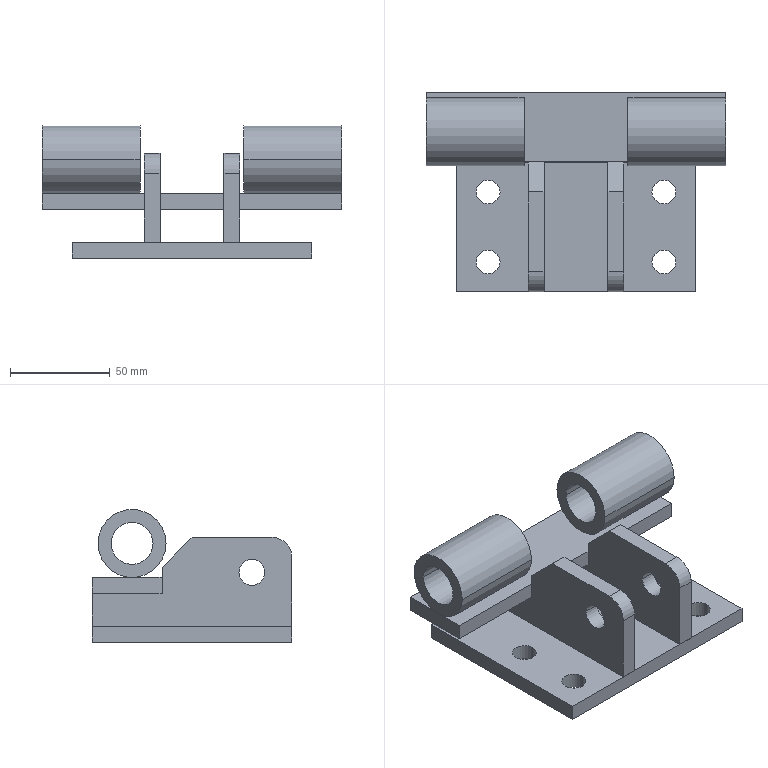Part | SolidWorks | features ICE 6, Chamfer 2, Fillet 2, MoveCopyBody 2, Extrusion 1, MirrorSolid 1, MoveFace 1 | 6 solids | 56 faces | box 150 x 100 x 66.5 mm | volume 240667 mm3 | plane 34 | cylinder 22 | commonest cylinder face diameters 12 x8 13 x4 21 x4 34 x4 20 x2
STEP:
#1=CARTESIAN_POINT('',(-75.,50.,32.5));
#2=VERTEX_POINT('',#1);
#3=CARTESIAN_POINT('',(-75.,15.,32.5));
#4=VERTEX_POINT('',#3);
#5=CARTESIAN_POINT('',(-75.,50.,32.5));
#6=DIRECTION('',(0.,-1.,0.));
#7=VECTOR('',#6,1000.);
#8=LINE('',#5,#7);
#9=EDGE_CURVE('',#2,#4,#8,.T.);
#10=ORIENTED_EDGE('',*,*,#9,.F.);
#11=CARTESIAN_POINT('',(-75.,50.,24.5));
#12=VERTEX_POINT('',#11);
#13=CARTESIAN_POINT('',(-75.,50.,24.5));
#14=DIRECTION('',(0.,0.,1.));
#15=VECTOR('',#14,1000.);
#16=LINE('',#13,#15);
#17=EDGE_CURVE('',#12,#2,#16,.T.);
#18=ORIENTED_EDGE('',*,*,#17,.F.);
#19=CARTESIAN_POINT('',(-75.,15.,24.5));
#20=VERTEX_POINT('',#19);
#21=CARTESIAN_POINT('',(-75.,50.,24.5));
#22=DIRECTION('',(0.,-1.,0.));
#23=VECTOR('',#22,1000.);
#24=LINE('',#21,#23);
#25=EDGE_CURVE('',#12,#20,#24,.T.);
#26=ORIENTED_EDGE('',*,*,#25,.T.);
#27=CARTESIAN_POINT('',(-75.,15.,24.5));
#28=DIRECTION('',(0.,0.,1.));
#29=VECTOR('',#28,1000.);
#30=LINE('',#27,#29);
#31=EDGE_CURVE('',#20,#4,#30,.T.);
#32=ORIENTED_EDGE('',*,*,#31,.T.);
#33=EDGE_LOOP('',(#10,#18,#26,#32));
#34=FACE_OUTER_BOUND('',#33,.T.);
#35=CARTESIAN_POINT('',(-75.,50.,24.5));
#36=DIRECTION('',(-1.,0.,0.));
#37=DIRECTION('',(0.,-1.,0.));
#38=AXIS2_PLACEMENT_3D('',#35,#36,#37);
#39=PLANE('',#38);
#40=ADVANCED_FACE('',(#34),#39,.T.);
#41=CARTESIAN_POINT('',(75.,50.,32.5));
#42=VERTEX_POINT('',#41);
#43=CARTESIAN_POINT('',(-75.,50.,32.5));
#44=DIRECTION('',(-1.,0.,0.));
#45=VECTOR('',#44,1000.);
#46=LINE('',#43,#45);
#47=EDGE_CURVE('',#42,#2,#46,.T.);
#48=ORIENTED_EDGE('',*,*,#47,.F.);
#49=CARTESIAN_POINT('',(75.,50.,24.5));
#50=VERTEX_POINT('',#49);
#51=CARTESIAN_POINT('',(75.,50.,24.5));
#52=DIRECTION('',(0.,0.,1.));
#53=VECTOR('',#52,1000.);
#54=LINE('',#51,#53);
#55=EDGE_CURVE('',#50,#42,#54,.T.);
#56=ORIENTED_EDGE('',*,*,#55,.F.);
#57=CARTESIAN_POINT('',(-75.,50.,24.5));
#58=DIRECTION('',(-1.,0.,0.));
#59=VECTOR('',#58,1000.);
#60=LINE('',#57,#59);
#61=EDGE_CURVE('',#50,#12,#60,.T.);
#62=ORIENTED_EDGE('',*,*,#61,.T.);
#63=ORIENTED_EDGE('',*,*,#17,.T.);
#64=EDGE_LOOP('',(#48,#56,#62,#63));
#65=FACE_OUTER_BOUND('',#64,.T.);
#66=CARTESIAN_POINT('',(-75.,50.,24.5));
#67=DIRECTION('',(0.,1.,0.));
#68=DIRECTION('',(0.,0.,1.));
#69=AXIS2_PLACEMENT_3D('',#66,#67,#68);
#70=PLANE('',#69);
#71=ADVANCED_FACE('',(#65),#70,.T.);
#72=CARTESIAN_POINT('',(75.,15.,32.5));
#73=VERTEX_POINT('',#72);
#74=CARTESIAN_POINT('',(75.,50.,32.5));
#75=DIRECTION('',(0.,1.,0.));
#76=VECTOR('',#75,1000.);
#77=LINE('',#74,#76);
#78=EDGE_CURVE('',#73,#42,#77,.T.);
#79=ORIENTED_EDGE('',*,*,#78,.F.);
#80=CARTESIAN_POINT('',(75.,15.,24.5));
#81=VERTEX_POINT('',#80);
#82=CARTESIAN_POINT('',(75.,15.,24.5));
#83=DIRECTION('',(0.,0.,1.));
#84=VECTOR('',#83,1000.);
#85=LINE('',#82,#84);
#86=EDGE_CURVE('',#81,#73,#85,.T.);
#87=ORIENTED_EDGE('',*,*,#86,.F.);
#88=CARTESIAN_POINT('',(75.,50.,24.5));
#89=DIRECTION('',(0.,1.,0.));
#90=VECTOR('',#89,1000.);
#91=LINE('',#88,#90);
#92=EDGE_CURVE('',#81,#50,#91,.T.);
#93=ORIENTED_EDGE('',*,*,#92,.T.);
#94=ORIENTED_EDGE('',*,*,#55,.T.);
#95=EDGE_LOOP('',(#79,#87,#93,#94));
#96=FACE_OUTER_BOUND('',#95,.T.);
#97=CARTESIAN_POINT('',(75.,50.,24.5));
#98=DIRECTION('',(1.,0.,0.));
#99=DIRECTION('',(0.,1.,0.));
#100=AXIS2_PLACEMENT_3D('',#97,#98,#99);
#101=PLANE('',#100);
#102=ADVANCED_FACE('',(#96),#101,.T.);
#103=CARTESIAN_POINT('',(-75.,15.,32.5));
#104=DIRECTION('',(1.,0.,0.));
#105=VECTOR('',#104,1000.);
#106=LINE('',#103,#105);
#107=EDGE_CURVE('',#4,#73,#106,.T.);
#108=ORIENTED_EDGE('',*,*,#107,.F.);
#109=ORIENTED_EDGE('',*,*,#31,.F.);
#110=CARTESIAN_POINT('',(-75.,15.,24.5));
#111=DIRECTION('',(1.,0.,0.));
#112=VECTOR('',#111,1000.);
#113=LINE('',#110,#112);
#114=EDGE_CURVE('',#20,#81,#113,.T.);
#115=ORIENTED_EDGE('',*,*,#114,.T.);
#116=ORIENTED_EDGE('',*,*,#86,.T.);
#117=EDGE_LOOP('',(#108,#109,#115,#116));
#118=FACE_OUTER_BOUND('',#117,.T.);
#119=CARTESIAN_POINT('',(-75.,15.,24.5));
#120=DIRECTION('',(0.,-1.,0.));
#121=DIRECTION('',(0.,0.,-1.));
#122=AXIS2_PLACEMENT_3D('',#119,#120,#121);
#123=PLANE('',#122);
#124=ADVANCED_FACE('',(#118),#123,.T.);
#125=ORIENTED_EDGE('',*,*,#25,.F.);
#126=ORIENTED_EDGE('',*,*,#61,.F.);
#127=ORIENTED_EDGE('',*,*,#92,.F.);
#128=ORIENTED_EDGE('',*,*,#114,.F.);
#129=EDGE_LOOP('',(#125,#126,#127,#128));
#130=FACE_OUTER_BOUND('',#129,.T.);
#131=CARTESIAN_POINT('',(0.,0.,24.5));
#132=DIRECTION('',(0.,0.,1.));
#133=DIRECTION('',(1.,0.,0.));
#134=AXIS2_PLACEMENT_3D('',#131,#132,#133);
#135=PLANE('',#134);
#136=ADVANCED_FACE('',(#130),#135,.F.);
#137=ORIENTED_EDGE('',*,*,#9,.T.);
#138=ORIENTED_EDGE('',*,*,#107,.T.);
#139=ORIENTED_EDGE('',*,*,#78,.T.);
#140=ORIENTED_EDGE('',*,*,#47,.T.);
#141=EDGE_LOOP('',(#137,#138,#139,#140));
#142=FACE_OUTER_BOUND('',#141,.T.);
#143=CARTESIAN_POINT('',(0.,0.,32.5));
#144=DIRECTION('',(0.,0.,1.));
#145=DIRECTION('',(1.,0.,0.));
#146=AXIS2_PLACEMENT_3D('',#143,#144,#145);
#147=PLANE('',#146);
#148=ADVANCED_FACE('',(#142),#147,.T.);
#149=CLOSED_SHELL('',(#40,#71,#102,#124,#136,#148));
#150=MANIFOLD_SOLID_BREP('',#149);
#151=CARTESIAN_POINT('',(16.,-36.5,35.));
#152=VERTEX_POINT('',#151);
#153=CARTESIAN_POINT('',(16.,-23.5,35.));
#154=VERTEX_POINT('',#153);
#155=CARTESIAN_POINT('',(16.,-30.,35.));
#156=DIRECTION('',(1.,0.,0.));
#157=DIRECTION('',(0.,1.,0.));
#158=AXIS2_PLACEMENT_3D('',#155,#156,#157);
#159=CIRCLE('',#158,6.5);
#160=EDGE_CURVE('',#152,#154,#159,.T.);
#161=ORIENTED_EDGE('',*,*,#160,.F.);
#162=CARTESIAN_POINT('',(24.,-36.5,35.));
#163=VERTEX_POINT('',#162);
#164=CARTESIAN_POINT('',(-71.,-36.5,35.));
#165=DIRECTION('',(1.,0.,0.));
#166=VECTOR('',#165,1000.);
#167=LINE('',#164,#166);
#168=EDGE_CURVE('',#152,#163,#167,.T.);
#169=ORIENTED_EDGE('',*,*,#168,.T.);
#170=CARTESIAN_POINT('',(24.,-23.5,35.));
#171=VERTEX_POINT('',#170);
#172=CARTESIAN_POINT('',(24.,-30.,35.));
#173=DIRECTION('',(1.,0.,0.));
#174=DIRECTION('',(0.,1.,0.));
#175=AXIS2_PLACEMENT_3D('',#172,#173,#174);
#176=CIRCLE('',#175,6.5);
#177=EDGE_CURVE('',#163,#171,#176,.T.);
#178=ORIENTED_EDGE('',*,*,#177,.T.);
#179=CARTESIAN_POINT('',(-71.,-23.5,35.));
#180=DIRECTION('',(1.,0.,0.));
#181=VECTOR('',#180,1000.);
#182=LINE('',#179,#181);
#183=EDGE_CURVE('',#154,#171,#182,.T.);
#184=ORIENTED_EDGE('',*,*,#183,.F.);
#185=EDGE_LOOP('',(#161,#169,#178,#184));
#186=FACE_OUTER_BOUND('',#185,.T.);
#187=CARTESIAN_POINT('',(-71.,-30.,35.));
#188=DIRECTION('',(1.,0.,0.));
#189=DIRECTION('',(0.,1.,0.));
#190=AXIS2_PLACEMENT_3D('',#187,#188,#189);
#191=CYLINDRICAL_SURFACE('',#190,6.5);
#192=ADVANCED_FACE('',(#186),#191,.F.);
#193=CARTESIAN_POINT('',(24.,-30.,35.));
#194=DIRECTION('',(1.,0.,0.));
#195=DIRECTION('',(0.,1.,0.));
#196=AXIS2_PLACEMENT_3D('',#193,#194,#195);
#197=CIRCLE('',#196,6.5);
#198=EDGE_CURVE('',#171,#163,#197,.T.);
#199=ORIENTED_EDGE('',*,*,#198,.F.);
#200=ORIENTED_EDGE('',*,*,#177,.F.);
#201=EDGE_LOOP('',(#199,#200));
#202=FACE_BOUND('',#201,.T.);
#203=CARTESIAN_POINT('',(24.,15.,37.5));
#204=VERTEX_POINT('',#203);
#205=CARTESIAN_POINT('',(24.,15.,24.5));
#206=VERTEX_POINT('',#205);
#207=CARTESIAN_POINT('',(24.,15.,32.5));
#208=DIRECTION('',(0.,0.,-1.));
#209=VECTOR('',#208,1000.);
#210=LINE('',#207,#209);
#211=EDGE_CURVE('',#204,#206,#210,.T.);
#212=ORIENTED_EDGE('',*,*,#211,.F.);
#213=CARTESIAN_POINT('',(24.,0.,52.5));
#214=VERTEX_POINT('',#213);
#215=CARTESIAN_POINT('',(24.,0.,52.5));
#216=DIRECTION('',(0.,-0.7071,0.7071));
#217=VECTOR('',#216,1000.);
#218=LINE('',#215,#217);
#219=EDGE_CURVE('',#204,#214,#218,.T.);
#220=ORIENTED_EDGE('',*,*,#219,.T.);
#221=CARTESIAN_POINT('',(24.,-40.,52.5));
#222=VERTEX_POINT('',#221);
#223=CARTESIAN_POINT('',(24.,0.,52.5));
#224=DIRECTION('',(0.,1.,0.));
#225=VECTOR('',#224,1000.);
#226=LINE('',#223,#225);
#227=EDGE_CURVE('',#222,#214,#226,.T.);
#228=ORIENTED_EDGE('',*,*,#227,.F.);
#229=CARTESIAN_POINT('',(24.,-50.,42.5));
#230=VERTEX_POINT('',#229);
#231=CARTESIAN_POINT('',(24.,-40.,42.5));
#232=DIRECTION('',(1.,0.,0.));
#233=DIRECTION('',(0.,-1.,0.));
#234=AXIS2_PLACEMENT_3D('',#231,#232,#233);
#235=CIRCLE('',#234,10.);
#236=EDGE_CURVE('',#222,#230,#235,.T.);
#237=ORIENTED_EDGE('',*,*,#236,.T.);
#238=CARTESIAN_POINT('',(24.,-50.,8.));
#239=VERTEX_POINT('',#238);
#240=CARTESIAN_POINT('',(24.,-50.,32.5));
#241=DIRECTION('',(0.,0.,-1.));
#242=VECTOR('',#241,1000.);
#243=LINE('',#240,#242);
#244=EDGE_CURVE('',#230,#239,#243,.T.);
#245=ORIENTED_EDGE('',*,*,#244,.T.);
#246=CARTESIAN_POINT('',(24.,50.,8.));
#247=VERTEX_POINT('',#246);
#248=CARTESIAN_POINT('',(24.,50.,8.));
#249=DIRECTION('',(0.,1.,0.));
#250=VECTOR('',#249,1000.);
#251=LINE('',#248,#250);
#252=EDGE_CURVE('',#239,#247,#251,.T.);
#253=ORIENTED_EDGE('',*,*,#252,.T.);
#254=CARTESIAN_POINT('',(24.,50.,24.5));
#255=VERTEX_POINT('',#254);
#256=CARTESIAN_POINT('',(24.,50.,32.5));
#257=DIRECTION('',(0.,0.,-1.));
#258=VECTOR('',#257,1000.);
#259=LINE('',#256,#258);
#260=EDGE_CURVE('',#255,#247,#259,.T.);
#261=ORIENTED_EDGE('',*,*,#260,.F.);
#262=CARTESIAN_POINT('',(24.,50.,24.5));
#263=DIRECTION('',(0.,1.,0.));
#264=VECTOR('',#263,1000.);
#265=LINE('',#262,#264);
#266=EDGE_CURVE('',#206,#255,#265,.T.);
#267=ORIENTED_EDGE('',*,*,#266,.F.);
#268=EDGE_LOOP('',(#212,#220,#228,#237,#245,#253,#261,#267));
#269=FACE_OUTER_BOUND('',#268,.T.);
#270=CARTESIAN_POINT('',(24.,50.,32.5));
#271=DIRECTION('',(-1.,0.,0.));
#272=DIRECTION('',(0.,-1.,0.));
#273=AXIS2_PLACEMENT_3D('',#270,#271,#272);
#274=PLANE('',#273);
#275=ADVANCED_FACE('',(#202,#269),#274,.F.);
#276=CARTESIAN_POINT('',(16.,50.,24.5));
#277=VERTEX_POINT('',#276);
#278=CARTESIAN_POINT('',(16.,50.,8.));
#279=VERTEX_POINT('',#278);
#280=CARTESIAN_POINT('',(16.,50.,32.5));
#281=DIRECTION('',(0.,0.,-1.));
#282=VECTOR('',#281,1000.);
#283=LINE('',#280,#282);
#284=EDGE_CURVE('',#277,#279,#283,.T.);
#285=ORIENTED_EDGE('',*,*,#284,.F.);
#286=CARTESIAN_POINT('',(-48.,50.,24.5));
#287=DIRECTION('',(1.,0.,0.));
#288=VECTOR('',#287,1000.);
#289=LINE('',#286,#288);
#290=EDGE_CURVE('',#277,#255,#289,.T.);
#291=ORIENTED_EDGE('',*,*,#290,.T.);
#292=ORIENTED_EDGE('',*,*,#260,.T.);
#293=CARTESIAN_POINT('',(24.,50.,8.));
#294=DIRECTION('',(-1.,0.,0.));
#295=VECTOR('',#294,1000.);
#296=LINE('',#293,#295);
#297=EDGE_CURVE('',#247,#279,#296,.T.);
#298=ORIENTED_EDGE('',*,*,#297,.T.);
#299=EDGE_LOOP('',(#285,#291,#292,#298));
#300=FACE_OUTER_BOUND('',#299,.T.);
#301=CARTESIAN_POINT('',(24.,50.,32.5));
#302=DIRECTION('',(0.,-1.,0.));
#303=DIRECTION('',(1.,0.,0.));
#304=AXIS2_PLACEMENT_3D('',#301,#302,#303);
#305=PLANE('',#304);
#306=ADVANCED_FACE('',(#300),#305,.F.);
#307=CARTESIAN_POINT('',(16.,-30.,35.));
#308=DIRECTION('',(1.,0.,0.));
#309=DIRECTION('',(0.,1.,0.));
#310=AXIS2_PLACEMENT_3D('',#307,#308,#309);
#311=CIRCLE('',#310,6.5);
#312=EDGE_CURVE('',#154,#152,#311,.T.);
#313=ORIENTED_EDGE('',*,*,#312,.T.);
#314=ORIENTED_EDGE('',*,*,#160,.T.);
#315=EDGE_LOOP('',(#313,#314));
#316=FACE_BOUND('',#315,.T.);
#317=CARTESIAN_POINT('',(16.,0.,52.5));
#318=VERTEX_POINT('',#317);
#319=CARTESIAN_POINT('',(16.,-40.,52.5));
#320=VERTEX_POINT('',#319);
#321=CARTESIAN_POINT('',(16.,0.,52.5));
#322=DIRECTION('',(0.,-1.,0.));
#323=VECTOR('',#322,1000.);
#324=LINE('',#321,#323);
#325=EDGE_CURVE('',#318,#320,#324,.T.);
#326=ORIENTED_EDGE('',*,*,#325,.F.);
#327=CARTESIAN_POINT('',(16.,15.,37.5));
#328=VERTEX_POINT('',#327);
#329=CARTESIAN_POINT('',(16.,0.,52.5));
#330=DIRECTION('',(0.,0.7071,-0.7071));
#331=VECTOR('',#330,1000.);
#332=LINE('',#329,#331);
#333=EDGE_CURVE('',#318,#328,#332,.T.);
#334=ORIENTED_EDGE('',*,*,#333,.T.);
#335=CARTESIAN_POINT('',(16.,15.,24.5));
#336=VERTEX_POINT('',#335);
#337=CARTESIAN_POINT('',(16.,15.,32.5));
#338=DIRECTION('',(0.,0.,-1.));
#339=VECTOR('',#338,1000.);
#340=LINE('',#337,#339);
#341=EDGE_CURVE('',#328,#336,#340,.T.);
#342=ORIENTED_EDGE('',*,*,#341,.T.);
#343=CARTESIAN_POINT('',(16.,50.,24.5));
#344=DIRECTION('',(0.,1.,0.));
#345=VECTOR('',#344,1000.);
#346=LINE('',#343,#345);
#347=EDGE_CURVE('',#336,#277,#346,.T.);
#348=ORIENTED_EDGE('',*,*,#347,.T.);
#349=ORIENTED_EDGE('',*,*,#284,.T.);
#350=CARTESIAN_POINT('',(16.,-50.,8.));
#351=VERTEX_POINT('',#350);
#352=CARTESIAN_POINT('',(16.,50.,8.));
#353=DIRECTION('',(0.,-1.,0.));
#354=VECTOR('',#353,1000.);
#355=LINE('',#352,#354);
#356=EDGE_CURVE('',#279,#351,#355,.T.);
#357=ORIENTED_EDGE('',*,*,#356,.T.);
#358=CARTESIAN_POINT('',(16.,-50.,42.5));
#359=VERTEX_POINT('',#358);
#360=CARTESIAN_POINT('',(16.,-50.,32.5));
#361=DIRECTION('',(0.,0.,-1.));
#362=VECTOR('',#361,1000.);
#363=LINE('',#360,#362);
#364=EDGE_CURVE('',#359,#351,#363,.T.);
#365=ORIENTED_EDGE('',*,*,#364,.F.);
#366=CARTESIAN_POINT('',(16.,-40.,42.5));
#367=DIRECTION('',(-1.,0.,0.));
#368=DIRECTION('',(0.,1.,0.));
#369=AXIS2_PLACEMENT_3D('',#366,#367,#368);
#370=CIRCLE('',#369,10.);
#371=EDGE_CURVE('',#359,#320,#370,.T.);
#372=ORIENTED_EDGE('',*,*,#371,.T.);
#373=EDGE_LOOP('',(#326,#334,#342,#348,#349,#357,#365,#372));
#374=FACE_OUTER_BOUND('',#373,.T.);
#375=CARTESIAN_POINT('',(16.,50.,32.5));
#376=DIRECTION('',(1.,0.,0.));
#377=DIRECTION('',(0.,1.,0.));
#378=AXIS2_PLACEMENT_3D('',#375,#376,#377);
#379=PLANE('',#378);
#380=ADVANCED_FACE('',(#316,#374),#379,.F.);
#381=ORIENTED_EDGE('',*,*,#244,.F.);
#382=CARTESIAN_POINT('',(24.,-50.,42.5));
#383=DIRECTION('',(-1.,0.,0.));
#384=VECTOR('',#383,1000.);
#385=LINE('',#382,#384);
#386=EDGE_CURVE('',#230,#359,#385,.T.);
#387=ORIENTED_EDGE('',*,*,#386,.T.);
#388=ORIENTED_EDGE('',*,*,#364,.T.);
#389=CARTESIAN_POINT('',(24.,-50.,8.));
#390=DIRECTION('',(1.,0.,0.));
#391=VECTOR('',#390,1000.);
#392=LINE('',#389,#391);
#393=EDGE_CURVE('',#351,#239,#392,.T.);
#394=ORIENTED_EDGE('',*,*,#393,.T.);
#395=EDGE_LOOP('',(#381,#387,#388,#394));
#396=FACE_OUTER_BOUND('',#395,.T.);
#397=CARTESIAN_POINT('',(24.,-50.,32.5));
#398=DIRECTION('',(0.,1.,0.));
#399=DIRECTION('',(-1.,0.,0.));
#400=AXIS2_PLACEMENT_3D('',#397,#398,#399);
#401=PLANE('',#400);
#402=ADVANCED_FACE('',(#396),#401,.F.);
#403=ORIENTED_EDGE('',*,*,#227,.T.);
#404=CARTESIAN_POINT('',(0.,0.,52.5));
#405=DIRECTION('',(-1.,0.,0.));
#406=VECTOR('',#405,1000.);
#407=LINE('',#404,#406);
#408=EDGE_CURVE('',#214,#318,#407,.T.);
#409=ORIENTED_EDGE('',*,*,#408,.T.);
#410=ORIENTED_EDGE('',*,*,#325,.T.);
#411=CARTESIAN_POINT('',(0.,-40.,52.5));
#412=DIRECTION('',(1.,0.,0.));
#413=VECTOR('',#412,1000.);
#414=LINE('',#411,#413);
#415=EDGE_CURVE('',#320,#222,#414,.T.);
#416=ORIENTED_EDGE('',*,*,#415,.T.);
#417=EDGE_LOOP('',(#403,#409,#410,#416));
#418=FACE_OUTER_BOUND('',#417,.T.);
#419=CARTESIAN_POINT('',(0.,0.,52.5));
#420=DIRECTION('',(0.,0.,-1.));
#421=DIRECTION('',(-1.,0.,0.));
#422=AXIS2_PLACEMENT_3D('',#419,#420,#421);
#423=PLANE('',#422);
#424=ADVANCED_FACE('',(#418),#423,.F.);
#425=ORIENTED_EDGE('',*,*,#252,.F.);
#426=ORIENTED_EDGE('',*,*,#393,.F.);
#427=ORIENTED_EDGE('',*,*,#356,.F.);
#428=ORIENTED_EDGE('',*,*,#297,.F.);
#429=EDGE_LOOP('',(#425,#426,#427,#428));
#430=FACE_OUTER_BOUND('',#429,.T.);
#431=CARTESIAN_POINT('',(0.,0.,8.));
#432=DIRECTION('',(0.,0.,-1.));
#433=DIRECTION('',(-1.,0.,0.));
#434=AXIS2_PLACEMENT_3D('',#431,#432,#433);
#435=PLANE('',#434);
#436=ADVANCED_FACE('',(#430),#435,.T.);
#437=CARTESIAN_POINT('',(-48.,15.,24.5));
#438=DIRECTION('',(1.,0.,0.));
#439=VECTOR('',#438,1000.);
#440=LINE('',#437,#439);
#441=EDGE_CURVE('',#336,#206,#440,.T.);
#442=ORIENTED_EDGE('',*,*,#441,.T.);
#443=ORIENTED_EDGE('',*,*,#266,.T.);
#444=ORIENTED_EDGE('',*,*,#290,.F.);
#445=ORIENTED_EDGE('',*,*,#347,.F.);
#446=EDGE_LOOP('',(#442,#443,#444,#445));
#447=FACE_OUTER_BOUND('',#446,.T.);
#448=CARTESIAN_POINT('',(-48.,50.,24.5));
#449=DIRECTION('',(0.,0.,-1.));
#450=DIRECTION('',(-1.,0.,0.));
#451=AXIS2_PLACEMENT_3D('',#448,#449,#450);
#452=PLANE('',#451);
#453=ADVANCED_FACE('',(#447),#452,.F.);
#454=ORIENTED_EDGE('',*,*,#341,.F.);
#455=CARTESIAN_POINT('',(-48.,15.,37.5));
#456=DIRECTION('',(1.,0.,0.));
#457=VECTOR('',#456,1000.);
#458=LINE('',#455,#457);
#459=EDGE_CURVE('',#328,#204,#458,.T.);
#460=ORIENTED_EDGE('',*,*,#459,.T.);
#461=ORIENTED_EDGE('',*,*,#211,.T.);
#462=ORIENTED_EDGE('',*,*,#441,.F.);
#463=EDGE_LOOP('',(#454,#460,#461,#462));
#464=FACE_OUTER_BOUND('',#463,.T.);
#465=CARTESIAN_POINT('',(-48.,15.,32.5));
#466=DIRECTION('',(0.,-1.,0.));
#467=DIRECTION('',(1.,0.,0.));
#468=AXIS2_PLACEMENT_3D('',#465,#466,#467);
#469=PLANE('',#468);
#470=ADVANCED_FACE('',(#464),#469,.F.);
#471=ORIENTED_EDGE('',*,*,#168,.F.);
#472=ORIENTED_EDGE('',*,*,#312,.F.);
#473=ORIENTED_EDGE('',*,*,#183,.T.);
#474=ORIENTED_EDGE('',*,*,#198,.T.);
#475=EDGE_LOOP('',(#471,#472,#473,#474));
#476=FACE_OUTER_BOUND('',#475,.T.);
#477=CARTESIAN_POINT('',(-71.,-30.,35.));
#478=DIRECTION('',(1.,0.,0.));
#479=DIRECTION('',(0.,1.,0.));
#480=AXIS2_PLACEMENT_3D('',#477,#478,#479);
#481=CYLINDRICAL_SURFACE('',#480,6.5);
#482=ADVANCED_FACE('',(#476),#481,.F.);
#483=ORIENTED_EDGE('',*,*,#371,.F.);
#484=ORIENTED_EDGE('',*,*,#386,.F.);
#485=ORIENTED_EDGE('',*,*,#236,.F.);
#486=ORIENTED_EDGE('',*,*,#415,.F.);
#487=EDGE_LOOP('',(#483,#484,#485,#486));
#488=FACE_OUTER_BOUND('',#487,.T.);
#489=CARTESIAN_POINT('',(0.,-40.,42.5));
#490=DIRECTION('',(1.,0.,0.));
#491=DIRECTION('',(0.,1.,0.));
#492=AXIS2_PLACEMENT_3D('',#489,#490,#491);
#493=CYLINDRICAL_SURFACE('',#492,10.);
#494=ADVANCED_FACE('',(#488),#493,.T.);
#495=ORIENTED_EDGE('',*,*,#219,.F.);
#496=ORIENTED_EDGE('',*,*,#459,.F.);
#497=ORIENTED_EDGE('',*,*,#333,.F.);
#498=ORIENTED_EDGE('',*,*,#408,.F.);
#499=EDGE_LOOP('',(#495,#496,#497,#498));
#500=FACE_OUTER_BOUND('',#499,.T.);
#501=CARTESIAN_POINT('',(0.,0.,52.5));
#502=DIRECTION('',(0.,-0.7071,-0.7071));
#503=DIRECTION('',(-1.,0.,0.));
#504=AXIS2_PLACEMENT_3D('',#501,#502,#503);
#505=PLANE('',#504);
#506=ADVANCED_FACE('',(#500),#505,.F.);
#507=CLOSED_SHELL('',(#192,#275,#306,#380,#402,#424,#436,#453,#470,#482,#494,#506));
#508=MANIFOLD_SOLID_BREP('',#507);
#509=CARTESIAN_POINT('',(-24.,-36.5,35.));
#510=VERTEX_POINT('',#509);
#511=CARTESIAN_POINT('',(-24.,-23.5,35.));
#512=VERTEX_POINT('',#511);
#513=CARTESIAN_POINT('',(-24.,-30.,35.));
#514=DIRECTION('',(1.,0.,0.));
#515=DIRECTION('',(0.,1.,0.));
#516=AXIS2_PLACEMENT_3D('',#513,#514,#515);
#517=CIRCLE('',#516,6.5);
#518=EDGE_CURVE('',#510,#512,#517,.T.);
#519=ORIENTED_EDGE('',*,*,#518,.F.);
#520=CARTESIAN_POINT('',(-16.,-36.5,35.));
#521=VERTEX_POINT('',#520);
#522=CARTESIAN_POINT('',(-71.,-36.5,35.));
#523=DIRECTION('',(1.,0.,0.));
#524=VECTOR('',#523,1000.);
#525=LINE('',#522,#524);
#526=EDGE_CURVE('',#510,#521,#525,.T.);
#527=ORIENTED_EDGE('',*,*,#526,.T.);
#528=CARTESIAN_POINT('',(-16.,-23.5,35.));
#529=VERTEX_POINT('',#528);
#530=CARTESIAN_POINT('',(-16.,-30.,35.));
#531=DIRECTION('',(-1.,0.,0.));
#532=DIRECTION('',(0.,-1.,0.));
#533=AXIS2_PLACEMENT_3D('',#530,#531,#532);
#534=CIRCLE('',#533,6.5);
#535=EDGE_CURVE('',#529,#521,#534,.T.);
#536=ORIENTED_EDGE('',*,*,#535,.F.);
#537=CARTESIAN_POINT('',(-71.,-23.5,35.));
#538=DIRECTION('',(1.,0.,0.));
#539=VECTOR('',#538,1000.);
#540=LINE('',#537,#539);
#541=EDGE_CURVE('',#512,#529,#540,.T.);
#542=ORIENTED_EDGE('',*,*,#541,.F.);
#543=EDGE_LOOP('',(#519,#527,#536,#542));
#544=FACE_OUTER_BOUND('',#543,.T.);
#545=CARTESIAN_POINT('',(-71.,-30.,35.));
#546=DIRECTION('',(1.,0.,0.));
#547=DIRECTION('',(0.,1.,0.));
#548=AXIS2_PLACEMENT_3D('',#545,#546,#547);
#549=CYLINDRICAL_SURFACE('',#548,6.5);
#550=ADVANCED_FACE('',(#544),#549,.F.);
#551=CARTESIAN_POINT('',(-24.,-30.,35.));
#552=DIRECTION('',(1.,0.,0.));
#553=DIRECTION('',(0.,1.,0.));
#554=AXIS2_PLACEMENT_3D('',#551,#552,#553);
#555=CIRCLE('',#554,6.5);
#556=EDGE_CURVE('',#512,#510,#555,.T.);
#557=ORIENTED_EDGE('',*,*,#556,.T.);
#558=ORIENTED_EDGE('',*,*,#518,.T.);
#559=EDGE_LOOP('',(#557,#558));
#560=FACE_BOUND('',#559,.T.);
#561=CARTESIAN_POINT('',(-24.,0.,52.5));
#562=VERTEX_POINT('',#561);
#563=CARTESIAN_POINT('',(-24.,-40.,52.5));
#564=VERTEX_POINT('',#563);
#565=CARTESIAN_POINT('',(-24.,50.,52.5));
#566=DIRECTION('',(0.,-1.,0.));
#567=VECTOR('',#566,1000.);
#568=LINE('',#565,#567);
#569=EDGE_CURVE('',#562,#564,#568,.T.);
#570=ORIENTED_EDGE('',*,*,#569,.F.);
#571=CARTESIAN_POINT('',(-24.,15.,37.5));
#572=VERTEX_POINT('',#571);
#573=CARTESIAN_POINT('',(-24.,15.,37.5));
#574=DIRECTION('',(0.,0.7071,-0.7071));
#575=VECTOR('',#574,1000.);
#576=LINE('',#573,#575);
#577=EDGE_CURVE('',#562,#572,#576,.T.);
#578=ORIENTED_EDGE('',*,*,#577,.T.);
#579=CARTESIAN_POINT('',(-24.,15.,24.5));
#580=VERTEX_POINT('',#579);
#581=CARTESIAN_POINT('',(-24.,15.,32.5));
#582=DIRECTION('',(0.,0.,-1.));
#583=VECTOR('',#582,1000.);
#584=LINE('',#581,#583);
#585=EDGE_CURVE('',#572,#580,#584,.T.);
#586=ORIENTED_EDGE('',*,*,#585,.T.);
#587=CARTESIAN_POINT('',(-24.,50.,24.5));
#588=VERTEX_POINT('',#587);
#589=CARTESIAN_POINT('',(-24.,50.,24.5));
#590=DIRECTION('',(0.,1.,0.));
#591=VECTOR('',#590,1000.);
#592=LINE('',#589,#591);
#593=EDGE_CURVE('',#580,#588,#592,.T.);
#594=ORIENTED_EDGE('',*,*,#593,.T.);
#595=CARTESIAN_POINT('',(-24.,50.,8.));
#596=VERTEX_POINT('',#595);
#597=CARTESIAN_POINT('',(-24.,50.,32.5));
#598=DIRECTION('',(0.,0.,-1.));
#599=VECTOR('',#598,1000.);
#600=LINE('',#597,#599);
#601=EDGE_CURVE('',#588,#596,#600,.T.);
#602=ORIENTED_EDGE('',*,*,#601,.T.);
#603=CARTESIAN_POINT('',(-24.,-50.,8.));
#604=VERTEX_POINT('',#603);
#605=CARTESIAN_POINT('',(-24.,50.,8.));
#606=DIRECTION('',(0.,-1.,0.));
#607=VECTOR('',#606,1000.);
#608=LINE('',#605,#607);
#609=EDGE_CURVE('',#596,#604,#608,.T.);
#610=ORIENTED_EDGE('',*,*,#609,.T.);
#611=CARTESIAN_POINT('',(-24.,-50.,42.5));
#612=VERTEX_POINT('',#611);
#613=CARTESIAN_POINT('',(-24.,-50.,32.5));
#614=DIRECTION('',(0.,0.,-1.));
#615=VECTOR('',#614,1000.);
#616=LINE('',#613,#615);
#617=EDGE_CURVE('',#612,#604,#616,.T.);
#618=ORIENTED_EDGE('',*,*,#617,.F.);
#619=CARTESIAN_POINT('',(-24.,-40.,42.5));
#620=DIRECTION('',(-1.,0.,0.));
#621=DIRECTION('',(0.,1.,0.));
#622=AXIS2_PLACEMENT_3D('',#619,#620,#621);
#623=CIRCLE('',#622,10.);
#624=EDGE_CURVE('',#612,#564,#623,.T.);
#625=ORIENTED_EDGE('',*,*,#624,.T.);
#626=EDGE_LOOP('',(#570,#578,#586,#594,#602,#610,#618,#625));
#627=FACE_OUTER_BOUND('',#626,.T.);
#628=CARTESIAN_POINT('',(-24.,50.,32.5));
#629=DIRECTION('',(1.,0.,0.));
#630=DIRECTION('',(0.,1.,0.));
#631=AXIS2_PLACEMENT_3D('',#628,#629,#630);
#632=PLANE('',#631);
#633=ADVANCED_FACE('',(#560,#627),#632,.F.);
#634=CARTESIAN_POINT('',(-16.,-50.,42.5));
#635=VERTEX_POINT('',#634);
#636=CARTESIAN_POINT('',(-16.,-50.,8.));
#637=VERTEX_POINT('',#636);
#638=CARTESIAN_POINT('',(-16.,-50.,32.5));
#639=DIRECTION('',(0.,0.,-1.));
#640=VECTOR('',#639,1000.);
#641=LINE('',#638,#640);
#642=EDGE_CURVE('',#635,#637,#641,.T.);
#643=ORIENTED_EDGE('',*,*,#642,.F.);
#644=CARTESIAN_POINT('',(-24.,-50.,42.5));
#645=DIRECTION('',(-1.,0.,0.));
#646=VECTOR('',#645,1000.);
#647=LINE('',#644,#646);
#648=EDGE_CURVE('',#635,#612,#647,.T.);
#649=ORIENTED_EDGE('',*,*,#648,.T.);
#650=ORIENTED_EDGE('',*,*,#617,.T.);
#651=CARTESIAN_POINT('',(-24.,-50.,8.));
#652=DIRECTION('',(1.,0.,0.));
#653=VECTOR('',#652,1000.);
#654=LINE('',#651,#653);
#655=EDGE_CURVE('',#604,#637,#654,.T.);
#656=ORIENTED_EDGE('',*,*,#655,.T.);
#657=EDGE_LOOP('',(#643,#649,#650,#656));
#658=FACE_OUTER_BOUND('',#657,.T.);
#659=CARTESIAN_POINT('',(-24.,-50.,32.5));
#660=DIRECTION('',(0.,1.,0.));
#661=DIRECTION('',(0.,0.,1.));
#662=AXIS2_PLACEMENT_3D('',#659,#660,#661);
#663=PLANE('',#662);
#664=ADVANCED_FACE('',(#658),#663,.F.);
#665=ORIENTED_EDGE('',*,*,#535,.T.);
#666=CARTESIAN_POINT('',(-16.,-30.,35.));
#667=DIRECTION('',(-1.,0.,0.));
#668=DIRECTION('',(0.,-1.,0.));
#669=AXIS2_PLACEMENT_3D('',#666,#667,#668);
#670=CIRCLE('',#669,6.5);
#671=EDGE_CURVE('',#521,#529,#670,.T.);
#672=ORIENTED_EDGE('',*,*,#671,.T.);
#673=EDGE_LOOP('',(#665,#672));
#674=FACE_BOUND('',#673,.T.);
#675=CARTESIAN_POINT('',(-16.,15.,24.5));
#676=VERTEX_POINT('',#675);
#677=CARTESIAN_POINT('',(-16.,15.,37.5));
#678=VERTEX_POINT('',#677);
#679=CARTESIAN_POINT('',(-16.,15.,32.5));
#680=DIRECTION('',(0.,0.,1.));
#681=VECTOR('',#680,1000.);
#682=LINE('',#679,#681);
#683=EDGE_CURVE('',#676,#678,#682,.T.);
#684=ORIENTED_EDGE('',*,*,#683,.T.);
#685=CARTESIAN_POINT('',(-16.,0.,52.5));
#686=VERTEX_POINT('',#685);
#687=CARTESIAN_POINT('',(-16.,15.,37.5));
#688=DIRECTION('',(0.,-0.7071,0.7071));
#689=VECTOR('',#688,1000.);
#690=LINE('',#687,#689);
#691=EDGE_CURVE('',#678,#686,#690,.T.);
#692=ORIENTED_EDGE('',*,*,#691,.T.);
#693=CARTESIAN_POINT('',(-16.,-40.,52.5));
#694=VERTEX_POINT('',#693);
#695=CARTESIAN_POINT('',(-16.,50.,52.5));
#696=DIRECTION('',(0.,1.,0.));
#697=VECTOR('',#696,1000.);
#698=LINE('',#695,#697);
#699=EDGE_CURVE('',#694,#686,#698,.T.);
#700=ORIENTED_EDGE('',*,*,#699,.F.);
#701=CARTESIAN_POINT('',(-16.,-40.,42.5));
#702=DIRECTION('',(1.,0.,0.));
#703=DIRECTION('',(0.,-1.,0.));
#704=AXIS2_PLACEMENT_3D('',#701,#702,#703);
#705=CIRCLE('',#704,10.);
#706=EDGE_CURVE('',#694,#635,#705,.T.);
#707=ORIENTED_EDGE('',*,*,#706,.T.);
#708=ORIENTED_EDGE('',*,*,#642,.T.);
#709=CARTESIAN_POINT('',(-16.,50.,8.));
#710=VERTEX_POINT('',#709);
#711=CARTESIAN_POINT('',(-16.,50.,8.));
#712=DIRECTION('',(0.,1.,0.));
#713=VECTOR('',#712,1000.);
#714=LINE('',#711,#713);
#715=EDGE_CURVE('',#637,#710,#714,.T.);
#716=ORIENTED_EDGE('',*,*,#715,.T.);
#717=CARTESIAN_POINT('',(-16.,50.,24.5));
#718=VERTEX_POINT('',#717);
#719=CARTESIAN_POINT('',(-16.,50.,32.5));
#720=DIRECTION('',(0.,0.,-1.));
#721=VECTOR('',#720,1000.);
#722=LINE('',#719,#721);
#723=EDGE_CURVE('',#718,#710,#722,.T.);
#724=ORIENTED_EDGE('',*,*,#723,.F.);
#725=CARTESIAN_POINT('',(-16.,50.,24.5));
#726=DIRECTION('',(0.,-1.,0.));
#727=VECTOR('',#726,1000.);
#728=LINE('',#725,#727);
#729=EDGE_CURVE('',#718,#676,#728,.T.);
#730=ORIENTED_EDGE('',*,*,#729,.T.);
#731=EDGE_LOOP('',(#684,#692,#700,#707,#708,#716,#724,#730));
#732=FACE_OUTER_BOUND('',#731,.T.);
#733=CARTESIAN_POINT('',(-16.,50.,32.5));
#734=DIRECTION('',(-1.,0.,0.));
#735=DIRECTION('',(0.,-1.,0.));
#736=AXIS2_PLACEMENT_3D('',#733,#734,#735);
#737=PLANE('',#736);
#738=ADVANCED_FACE('',(#674,#732),#737,.F.);
#739=ORIENTED_EDGE('',*,*,#601,.F.);
#740=CARTESIAN_POINT('',(-48.,50.,24.5));
#741=DIRECTION('',(1.,0.,0.));
#742=VECTOR('',#741,1000.);
#743=LINE('',#740,#742);
#744=EDGE_CURVE('',#588,#718,#743,.T.);
#745=ORIENTED_EDGE('',*,*,#744,.T.);
#746=ORIENTED_EDGE('',*,*,#723,.T.);
#747=CARTESIAN_POINT('',(-24.,50.,8.));
#748=DIRECTION('',(-1.,0.,0.));
#749=VECTOR('',#748,1000.);
#750=LINE('',#747,#749);
#751=EDGE_CURVE('',#710,#596,#750,.T.);
#752=ORIENTED_EDGE('',*,*,#751,.T.);
#753=EDGE_LOOP('',(#739,#745,#746,#752));
#754=FACE_OUTER_BOUND('',#753,.T.);
#755=CARTESIAN_POINT('',(-24.,50.,32.5));
#756=DIRECTION('',(0.,-1.,0.));
#757=DIRECTION('',(1.,0.,0.));
#758=AXIS2_PLACEMENT_3D('',#755,#756,#757);
#759=PLANE('',#758);
#760=ADVANCED_FACE('',(#754),#759,.F.);
#761=ORIENTED_EDGE('',*,*,#699,.T.);
#762=CARTESIAN_POINT('',(-24.,0.,52.5));
#763=DIRECTION('',(-1.,0.,0.));
#764=VECTOR('',#763,1000.);
#765=LINE('',#762,#764);
#766=EDGE_CURVE('',#686,#562,#765,.T.);
#767=ORIENTED_EDGE('',*,*,#766,.T.);
#768=ORIENTED_EDGE('',*,*,#569,.T.);
#769=CARTESIAN_POINT('',(-16.,-40.,52.5));
#770=DIRECTION('',(1.,0.,0.));
#771=VECTOR('',#770,1000.);
#772=LINE('',#769,#771);
#773=EDGE_CURVE('',#564,#694,#772,.T.);
#774=ORIENTED_EDGE('',*,*,#773,.T.);
#775=EDGE_LOOP('',(#761,#767,#768,#774));
#776=FACE_OUTER_BOUND('',#775,.T.);
#777=CARTESIAN_POINT('',(0.,0.,52.5));
#778=DIRECTION('',(0.,0.,1.));
#779=DIRECTION('',(1.,0.,0.));
#780=AXIS2_PLACEMENT_3D('',#777,#778,#779);
#781=PLANE('',#780);
#782=ADVANCED_FACE('',(#776),#781,.T.);
#783=ORIENTED_EDGE('',*,*,#609,.F.);
#784=ORIENTED_EDGE('',*,*,#751,.F.);
#785=ORIENTED_EDGE('',*,*,#715,.F.);
#786=ORIENTED_EDGE('',*,*,#655,.F.);
#787=EDGE_LOOP('',(#783,#784,#785,#786));
#788=FACE_OUTER_BOUND('',#787,.T.);
#789=CARTESIAN_POINT('',(0.,0.,8.));
#790=DIRECTION('',(0.,0.,1.));
#791=DIRECTION('',(1.,0.,0.));
#792=AXIS2_PLACEMENT_3D('',#789,#790,#791);
#793=PLANE('',#792);
#794=ADVANCED_FACE('',(#788),#793,.F.);
#795=CARTESIAN_POINT('',(-48.,15.,24.5));
#796=DIRECTION('',(1.,0.,0.));
#797=VECTOR('',#796,1000.);
#798=LINE('',#795,#797);
#799=EDGE_CURVE('',#580,#676,#798,.T.);
#800=ORIENTED_EDGE('',*,*,#799,.T.);
#801=ORIENTED_EDGE('',*,*,#729,.F.);
#802=ORIENTED_EDGE('',*,*,#744,.F.);
#803=ORIENTED_EDGE('',*,*,#593,.F.);
#804=EDGE_LOOP('',(#800,#801,#802,#803));
#805=FACE_OUTER_BOUND('',#804,.T.);
#806=CARTESIAN_POINT('',(-48.,50.,24.5));
#807=DIRECTION('',(0.,0.,-1.));
#808=DIRECTION('',(-1.,0.,0.));
#809=AXIS2_PLACEMENT_3D('',#806,#807,#808);
#810=PLANE('',#809);
#811=ADVANCED_FACE('',(#805),#810,.F.);
#812=ORIENTED_EDGE('',*,*,#585,.F.);
#813=CARTESIAN_POINT('',(-16.,15.,37.5));
#814=DIRECTION('',(1.,0.,0.));
#815=VECTOR('',#814,1000.);
#816=LINE('',#813,#815);
#817=EDGE_CURVE('',#572,#678,#816,.T.);
#818=ORIENTED_EDGE('',*,*,#817,.T.);
#819=ORIENTED_EDGE('',*,*,#683,.F.);
#820=ORIENTED_EDGE('',*,*,#799,.F.);
#821=EDGE_LOOP('',(#812,#818,#819,#820));
#822=FACE_OUTER_BOUND('',#821,.T.);
#823=CARTESIAN_POINT('',(-48.,15.,32.5));
#824=DIRECTION('',(0.,-1.,0.));
#825=DIRECTION('',(1.,0.,0.));
#826=AXIS2_PLACEMENT_3D('',#823,#824,#825);
#827=PLANE('',#826);
#828=ADVANCED_FACE('',(#822),#827,.F.);
#829=ORIENTED_EDGE('',*,*,#526,.F.);
#830=ORIENTED_EDGE('',*,*,#556,.F.);
#831=ORIENTED_EDGE('',*,*,#541,.T.);
#832=ORIENTED_EDGE('',*,*,#671,.F.);
#833=EDGE_LOOP('',(#829,#830,#831,#832));
#834=FACE_OUTER_BOUND('',#833,.T.);
#835=CARTESIAN_POINT('',(-71.,-30.,35.));
#836=DIRECTION('',(1.,0.,0.));
#837=DIRECTION('',(0.,1.,0.));
#838=AXIS2_PLACEMENT_3D('',#835,#836,#837);
#839=CYLINDRICAL_SURFACE('',#838,6.5);
#840=ADVANCED_FACE('',(#834),#839,.F.);
#841=ORIENTED_EDGE('',*,*,#624,.F.);
#842=ORIENTED_EDGE('',*,*,#648,.F.);
#843=ORIENTED_EDGE('',*,*,#706,.F.);
#844=ORIENTED_EDGE('',*,*,#773,.F.);
#845=EDGE_LOOP('',(#841,#842,#843,#844));
#846=FACE_OUTER_BOUND('',#845,.T.);
#847=CARTESIAN_POINT('',(0.,-40.,42.5));
#848=DIRECTION('',(-1.,0.,0.));
#849=DIRECTION('',(0.,0.,1.));
#850=AXIS2_PLACEMENT_3D('',#847,#848,#849);
#851=CYLINDRICAL_SURFACE('',#850,10.);
#852=ADVANCED_FACE('',(#846),#851,.T.);
#853=ORIENTED_EDGE('',*,*,#577,.F.);
#854=ORIENTED_EDGE('',*,*,#766,.F.);
#855=ORIENTED_EDGE('',*,*,#691,.F.);
#856=ORIENTED_EDGE('',*,*,#817,.F.);
#857=EDGE_LOOP('',(#853,#854,#855,#856));
#858=FACE_OUTER_BOUND('',#857,.T.);
#859=CARTESIAN_POINT('',(-48.,15.,37.5));
#860=DIRECTION('',(0.,0.7071,0.7071));
#861=DIRECTION('',(-1.,0.,0.));
#862=AXIS2_PLACEMENT_3D('',#859,#860,#861);
#863=PLANE('',#862);
#864=ADVANCED_FACE('',(#858),#863,.T.);
#865=CLOSED_SHELL('',(#550,#633,#664,#738,#760,#782,#794,#811,#828,#840,#852,#864));
#866=MANIFOLD_SOLID_BREP('',#865);
#867=CARTESIAN_POINT('',(38.,0.,0.));
#868=VERTEX_POINT('',#867);
#869=CARTESIAN_POINT('',(50.,0.,0.));
#870=VERTEX_POINT('',#869);
#871=CARTESIAN_POINT('',(44.,0.,0.));
#872=DIRECTION('',(0.,0.,1.));
#873=DIRECTION('',(1.,0.,0.));
#874=AXIS2_PLACEMENT_3D('',#871,#872,#873);
#875=CIRCLE('',#874,6.);
#876=EDGE_CURVE('',#868,#870,#875,.T.);
#877=ORIENTED_EDGE('',*,*,#876,.F.);
#878=CARTESIAN_POINT('',(38.,0.,8.));
#879=VERTEX_POINT('',#878);
#880=CARTESIAN_POINT('',(38.,0.,-2.));
#881=DIRECTION('',(0.,0.,1.));
#882=VECTOR('',#881,1000.);
#883=LINE('',#880,#882);
#884=EDGE_CURVE('',#868,#879,#883,.T.);
#885=ORIENTED_EDGE('',*,*,#884,.T.);
#886=CARTESIAN_POINT('',(50.,0.,8.));
#887=VERTEX_POINT('',#886);
#888=CARTESIAN_POINT('',(44.,0.,8.));
#889=DIRECTION('',(0.,0.,1.));
#890=DIRECTION('',(-1.,0.,0.));
#891=AXIS2_PLACEMENT_3D('',#888,#889,#890);
#892=CIRCLE('',#891,6.);
#893=EDGE_CURVE('',#879,#887,#892,.T.);
#894=ORIENTED_EDGE('',*,*,#893,.T.);
#895=CARTESIAN_POINT('',(50.,0.,-2.));
#896=DIRECTION('',(0.,0.,1.));
#897=VECTOR('',#896,1000.);
#898=LINE('',#895,#897);
#899=EDGE_CURVE('',#870,#887,#898,.T.);
#900=ORIENTED_EDGE('',*,*,#899,.F.);
#901=EDGE_LOOP('',(#877,#885,#894,#900));
#902=FACE_OUTER_BOUND('',#901,.T.);
#903=CARTESIAN_POINT('',(44.,0.,-2.));
#904=DIRECTION('',(0.,0.,1.));
#905=DIRECTION('',(1.,0.,0.));
#906=AXIS2_PLACEMENT_3D('',#903,#904,#905);
#907=CYLINDRICAL_SURFACE('',#906,6.);
#908=ADVANCED_FACE('',(#902),#907,.F.);
#909=CARTESIAN_POINT('',(38.,-35.,0.));
#910=VERTEX_POINT('',#909);
#911=CARTESIAN_POINT('',(50.,-35.,0.));
#912=VERTEX_POINT('',#911);
#913=CARTESIAN_POINT('',(44.,-35.,0.));
#914=DIRECTION('',(0.,0.,1.));
#915=DIRECTION('',(1.,0.,0.));
#916=AXIS2_PLACEMENT_3D('',#913,#914,#915);
#917=CIRCLE('',#916,6.);
#918=EDGE_CURVE('',#910,#912,#917,.T.);
#919=ORIENTED_EDGE('',*,*,#918,.F.);
#920=CARTESIAN_POINT('',(38.,-35.,8.));
#921=VERTEX_POINT('',#920);
#922=CARTESIAN_POINT('',(38.,-35.,-2.));
#923=DIRECTION('',(0.,0.,1.));
#924=VECTOR('',#923,1000.);
#925=LINE('',#922,#924);
#926=EDGE_CURVE('',#910,#921,#925,.T.);
#927=ORIENTED_EDGE('',*,*,#926,.T.);
#928=CARTESIAN_POINT('',(50.,-35.,8.));
#929=VERTEX_POINT('',#928);
#930=CARTESIAN_POINT('',(44.,-35.,8.));
#931=DIRECTION('',(0.,0.,1.));
#932=DIRECTION('',(-1.,0.,0.));
#933=AXIS2_PLACEMENT_3D('',#930,#931,#932);
#934=CIRCLE('',#933,6.);
#935=EDGE_CURVE('',#921,#929,#934,.T.);
#936=ORIENTED_EDGE('',*,*,#935,.T.);
#937=CARTESIAN_POINT('',(50.,-35.,-2.));
#938=DIRECTION('',(0.,0.,1.));
#939=VECTOR('',#938,1000.);
#940=LINE('',#937,#939);
#941=EDGE_CURVE('',#912,#929,#940,.T.);
#942=ORIENTED_EDGE('',*,*,#941,.F.);
#943=EDGE_LOOP('',(#919,#927,#936,#942));
#944=FACE_OUTER_BOUND('',#943,.T.);
#945=CARTESIAN_POINT('',(44.,-35.,-2.));
#946=DIRECTION('',(0.,0.,1.));
#947=DIRECTION('',(1.,0.,0.));
#948=AXIS2_PLACEMENT_3D('',#945,#946,#947);
#949=CYLINDRICAL_SURFACE('',#948,6.);
#950=ADVANCED_FACE('',(#944),#949,.F.);
#951=CARTESIAN_POINT('',(-50.,-35.,0.));
#952=VERTEX_POINT('',#951);
#953=CARTESIAN_POINT('',(-38.,-35.,0.));
#954=VERTEX_POINT('',#953);
#955=CARTESIAN_POINT('',(-44.,-35.,0.));
#956=DIRECTION('',(0.,0.,1.));
#957=DIRECTION('',(1.,0.,0.));
#958=AXIS2_PLACEMENT_3D('',#955,#956,#957);
#959=CIRCLE('',#958,6.);
#960=EDGE_CURVE('',#952,#954,#959,.T.);
#961=ORIENTED_EDGE('',*,*,#960,.F.);
#962=CARTESIAN_POINT('',(-50.,-35.,8.));
#963=VERTEX_POINT('',#962);
#964=CARTESIAN_POINT('',(-50.,-35.,-2.));
#965=DIRECTION('',(0.,0.,1.));
#966=VECTOR('',#965,1000.);
#967=LINE('',#964,#966);
#968=EDGE_CURVE('',#952,#963,#967,.T.);
#969=ORIENTED_EDGE('',*,*,#968,.T.);
#970=CARTESIAN_POINT('',(-38.,-35.,8.));
#971=VERTEX_POINT('',#970);
#972=CARTESIAN_POINT('',(-44.,-35.,8.));
#973=DIRECTION('',(0.,0.,1.));
#974=DIRECTION('',(1.,0.,0.));
#975=AXIS2_PLACEMENT_3D('',#972,#973,#974);
#976=CIRCLE('',#975,6.);
#977=EDGE_CURVE('',#963,#971,#976,.T.);
#978=ORIENTED_EDGE('',*,*,#977,.T.);
#979=CARTESIAN_POINT('',(-38.,-35.,-2.));
#980=DIRECTION('',(0.,0.,1.));
#981=VECTOR('',#980,1000.);
#982=LINE('',#979,#981);
#983=EDGE_CURVE('',#954,#971,#982,.T.);
#984=ORIENTED_EDGE('',*,*,#983,.F.);
#985=EDGE_LOOP('',(#961,#969,#978,#984));
#986=FACE_OUTER_BOUND('',#985,.T.);
#987=CARTESIAN_POINT('',(-44.,-35.,-2.));
#988=DIRECTION('',(0.,0.,1.));
#989=DIRECTION('',(1.,0.,0.));
#990=AXIS2_PLACEMENT_3D('',#987,#988,#989);
#991=CYLINDRICAL_SURFACE('',#990,6.);
#992=ADVANCED_FACE('',(#986),#991,.F.);
#993=CARTESIAN_POINT('',(-50.,0.,0.));
#994=VERTEX_POINT('',#993);
#995=CARTESIAN_POINT('',(-38.,0.,0.));
#996=VERTEX_POINT('',#995);
#997=CARTESIAN_POINT('',(-44.,0.,0.));
#998=DIRECTION('',(0.,0.,1.));
#999=DIRECTION('',(1.,0.,0.));
#1000=AXIS2_PLACEMENT_3D('',#997,#998,#999);
#1001=CIRCLE('',#1000,6.);
#1002=EDGE_CURVE('',#994,#996,#1001,.T.);
#1003=ORIENTED_EDGE('',*,*,#1002,.F.);
#1004=CARTESIAN_POINT('',(-50.,0.,8.));
#1005=VERTEX_POINT('',#1004);
#1006=CARTESIAN_POINT('',(-50.,0.,-2.));
#1007=DIRECTION('',(0.,0.,1.));
#1008=VECTOR('',#1007,1000.);
#1009=LINE('',#1006,#1008);
#1010=EDGE_CURVE('',#994,#1005,#1009,.T.);
#1011=ORIENTED_EDGE('',*,*,#1010,.T.);
#1012=CARTESIAN_POINT('',(-38.,0.,8.));
#1013=VERTEX_POINT('',#1012);
#1014=CARTESIAN_POINT('',(-44.,0.,8.));
#1015=DIRECTION('',(0.,0.,1.));
#1016=DIRECTION('',(1.,0.,0.));
#1017=AXIS2_PLACEMENT_3D('',#1014,#1015,#1016);
#1018=CIRCLE('',#1017,6.);
#1019=EDGE_CURVE('',#1005,#1013,#1018,.T.);
#1020=ORIENTED_EDGE('',*,*,#1019,.T.);
#1021=CARTESIAN_POINT('',(-38.,0.,-2.));
#1022=DIRECTION('',(0.,0.,1.));
#1023=VECTOR('',#1022,1000.);
#1024=LINE('',#1021,#1023);
#1025=EDGE_CURVE('',#996,#1013,#1024,.T.);
#1026=ORIENTED_EDGE('',*,*,#1025,.F.);
#1027=EDGE_LOOP('',(#1003,#1011,#1020,#1026));
#1028=FACE_OUTER_BOUND('',#1027,.T.);
#1029=CARTESIAN_POINT('',(-44.,0.,-2.));
#1030=DIRECTION('',(0.,0.,1.));
#1031=DIRECTION('',(1.,0.,0.));
#1032=AXIS2_PLACEMENT_3D('',#1029,#1030,#1031);
#1033=CYLINDRICAL_SURFACE('',#1032,6.);
#1034=ADVANCED_FACE('',(#1028),#1033,.F.);
#1035=CARTESIAN_POINT('',(60.,-50.,0.));
#1036=VERTEX_POINT('',#1035);
#1037=CARTESIAN_POINT('',(60.,50.,0.));
#1038=VERTEX_POINT('',#1037);
#1039=CARTESIAN_POINT('',(60.,50.,0.));
#1040=DIRECTION('',(0.,1.,0.));
#1041=VECTOR('',#1040,1000.);
#1042=LINE('',#1039,#1041);
#1043=EDGE_CURVE('',#1036,#1038,#1042,.T.);
#1044=ORIENTED_EDGE('',*,*,#1043,.T.);
#1045=CARTESIAN_POINT('',(60.,50.,8.));
#1046=VERTEX_POINT('',#1045);
#1047=CARTESIAN_POINT('',(60.,50.,8.));
#1048=DIRECTION('',(0.,0.,-1.));
#1049=VECTOR('',#1048,1000.);
#1050=LINE('',#1047,#1049);
#1051=EDGE_CURVE('',#1046,#1038,#1050,.T.);
#1052=ORIENTED_EDGE('',*,*,#1051,.F.);
#1053=CARTESIAN_POINT('',(60.,-50.,8.));
#1054=VERTEX_POINT('',#1053);
#1055=CARTESIAN_POINT('',(60.,50.,8.));
#1056=DIRECTION('',(0.,1.,0.));
#1057=VECTOR('',#1056,1000.);
#1058=LINE('',#1055,#1057);
#1059=EDGE_CURVE('',#1054,#1046,#1058,.T.);
#1060=ORIENTED_EDGE('',*,*,#1059,.F.);
#1061=CARTESIAN_POINT('',(60.,-50.,8.));
#1062=DIRECTION('',(0.,0.,-1.));
#1063=VECTOR('',#1062,1000.);
#1064=LINE('',#1061,#1063);
#1065=EDGE_CURVE('',#1054,#1036,#1064,.T.);
#1066=ORIENTED_EDGE('',*,*,#1065,.T.);
#1067=EDGE_LOOP('',(#1044,#1052,#1060,#1066));
#1068=FACE_OUTER_BOUND('',#1067,.T.);
#1069=CARTESIAN_POINT('',(60.,50.,8.));
#1070=DIRECTION('',(-1.,0.,0.));
#1071=DIRECTION('',(0.,-1.,0.));
#1072=AXIS2_PLACEMENT_3D('',#1069,#1070,#1071);
#1073=PLANE('',#1072);
#1074=ADVANCED_FACE('',(#1068),#1073,.F.);
#1075=CARTESIAN_POINT('',(-60.,50.,0.));
#1076=VERTEX_POINT('',#1075);
#1077=CARTESIAN_POINT('',(-60.,50.,0.));
#1078=DIRECTION('',(-1.,0.,0.));
#1079=VECTOR('',#1078,1000.);
#1080=LINE('',#1077,#1079);
#1081=EDGE_CURVE('',#1038,#1076,#1080,.T.);
#1082=ORIENTED_EDGE('',*,*,#1081,.T.);
#1083=CARTESIAN_POINT('',(-60.,50.,8.));
#1084=VERTEX_POINT('',#1083);
#1085=CARTESIAN_POINT('',(-60.,50.,8.));
#1086=DIRECTION('',(0.,0.,-1.));
#1087=VECTOR('',#1086,1000.);
#1088=LINE('',#1085,#1087);
#1089=EDGE_CURVE('',#1084,#1076,#1088,.T.);
#1090=ORIENTED_EDGE('',*,*,#1089,.F.);
#1091=CARTESIAN_POINT('',(-60.,50.,8.));
#1092=DIRECTION('',(-1.,0.,0.));
#1093=VECTOR('',#1092,1000.);
#1094=LINE('',#1091,#1093);
#1095=EDGE_CURVE('',#1046,#1084,#1094,.T.);
#1096=ORIENTED_EDGE('',*,*,#1095,.F.);
#1097=ORIENTED_EDGE('',*,*,#1051,.T.);
#1098=EDGE_LOOP('',(#1082,#1090,#1096,#1097));
#1099=FACE_OUTER_BOUND('',#1098,.T.);
#1100=CARTESIAN_POINT('',(-60.,50.,8.));
#1101=DIRECTION('',(0.,-1.,0.));
#1102=DIRECTION('',(0.,0.,-1.));
#1103=AXIS2_PLACEMENT_3D('',#1100,#1101,#1102);
#1104=PLANE('',#1103);
#1105=ADVANCED_FACE('',(#1099),#1104,.F.);
#1106=CARTESIAN_POINT('',(-60.,-50.,0.));
#1107=VERTEX_POINT('',#1106);
#1108=CARTESIAN_POINT('',(-60.,50.,0.));
#1109=DIRECTION('',(0.,-1.,0.));
#1110=VECTOR('',#1109,1000.);
#1111=LINE('',#1108,#1110);
#1112=EDGE_CURVE('',#1076,#1107,#1111,.T.);
#1113=ORIENTED_EDGE('',*,*,#1112,.T.);
#1114=CARTESIAN_POINT('',(-60.,-50.,8.));
#1115=VERTEX_POINT('',#1114);
#1116=CARTESIAN_POINT('',(-60.,-50.,8.));
#1117=DIRECTION('',(0.,0.,-1.));
#1118=VECTOR('',#1117,1000.);
#1119=LINE('',#1116,#1118);
#1120=EDGE_CURVE('',#1115,#1107,#1119,.T.);
#1121=ORIENTED_EDGE('',*,*,#1120,.F.);
#1122=CARTESIAN_POINT('',(-60.,50.,8.));
#1123=DIRECTION('',(0.,-1.,0.));
#1124=VECTOR('',#1123,1000.);
#1125=LINE('',#1122,#1124);
#1126=EDGE_CURVE('',#1084,#1115,#1125,.T.);
#1127=ORIENTED_EDGE('',*,*,#1126,.F.);
#1128=ORIENTED_EDGE('',*,*,#1089,.T.);
#1129=EDGE_LOOP('',(#1113,#1121,#1127,#1128));
#1130=FACE_OUTER_BOUND('',#1129,.T.);
#1131=CARTESIAN_POINT('',(-60.,50.,8.));
#1132=DIRECTION('',(1.,0.,0.));
#1133=DIRECTION('',(0.,1.,0.));
#1134=AXIS2_PLACEMENT_3D('',#1131,#1132,#1133);
#1135=PLANE('',#1134);
#1136=ADVANCED_FACE('',(#1130),#1135,.F.);
#1137=CARTESIAN_POINT('',(-60.,-50.,0.));
#1138=DIRECTION('',(1.,0.,0.));
#1139=VECTOR('',#1138,1000.);
#1140=LINE('',#1137,#1139);
#1141=EDGE_CURVE('',#1107,#1036,#1140,.T.);
#1142=ORIENTED_EDGE('',*,*,#1141,.T.);
#1143=ORIENTED_EDGE('',*,*,#1065,.F.);
#1144=CARTESIAN_POINT('',(-60.,-50.,8.));
#1145=DIRECTION('',(1.,0.,0.));
#1146=VECTOR('',#1145,1000.);
#1147=LINE('',#1144,#1146);
#1148=EDGE_CURVE('',#1115,#1054,#1147,.T.);
#1149=ORIENTED_EDGE('',*,*,#1148,.F.);
#1150=ORIENTED_EDGE('',*,*,#1120,.T.);
#1151=EDGE_LOOP('',(#1142,#1143,#1149,#1150));
#1152=FACE_OUTER_BOUND('',#1151,.T.);
#1153=CARTESIAN_POINT('',(-60.,-50.,8.));
#1154=DIRECTION('',(0.,1.,0.));
#1155=DIRECTION('',(0.,0.,1.));
#1156=AXIS2_PLACEMENT_3D('',#1153,#1154,#1155);
#1157=PLANE('',#1156);
#1158=ADVANCED_FACE('',(#1152),#1157,.F.);
#1159=CARTESIAN_POINT('',(44.,0.,8.));
#1160=DIRECTION('',(0.,0.,1.));
#1161=DIRECTION('',(-1.,0.,0.));
#1162=AXIS2_PLACEMENT_3D('',#1159,#1160,#1161);
#1163=CIRCLE('',#1162,6.);
#1164=EDGE_CURVE('',#887,#879,#1163,.T.);
#1165=ORIENTED_EDGE('',*,*,#1164,.F.);
#1166=ORIENTED_EDGE('',*,*,#893,.F.);
#1167=EDGE_LOOP('',(#1165,#1166));
#1168=FACE_BOUND('',#1167,.T.);
#1169=CARTESIAN_POINT('',(44.,-35.,8.));
#1170=DIRECTION('',(0.,0.,1.));
#1171=DIRECTION('',(-1.,0.,0.));
#1172=AXIS2_PLACEMENT_3D('',#1169,#1170,#1171);
#1173=CIRCLE('',#1172,6.);
#1174=EDGE_CURVE('',#929,#921,#1173,.T.);
#1175=ORIENTED_EDGE('',*,*,#1174,.F.);
#1176=ORIENTED_EDGE('',*,*,#935,.F.);
#1177=EDGE_LOOP('',(#1175,#1176));
#1178=FACE_BOUND('',#1177,.T.);
#1179=CARTESIAN_POINT('',(-44.,-35.,8.));
#1180=DIRECTION('',(0.,0.,1.));
#1181=DIRECTION('',(1.,0.,0.));
#1182=AXIS2_PLACEMENT_3D('',#1179,#1180,#1181);
#1183=CIRCLE('',#1182,6.);
#1184=EDGE_CURVE('',#971,#963,#1183,.T.);
#1185=ORIENTED_EDGE('',*,*,#1184,.F.);
#1186=ORIENTED_EDGE('',*,*,#977,.F.);
#1187=EDGE_LOOP('',(#1185,#1186));
#1188=FACE_BOUND('',#1187,.T.);
#1189=CARTESIAN_POINT('',(-44.,0.,8.));
#1190=DIRECTION('',(0.,0.,1.));
#1191=DIRECTION('',(1.,0.,0.));
#1192=AXIS2_PLACEMENT_3D('',#1189,#1190,#1191);
#1193=CIRCLE('',#1192,6.);
#1194=EDGE_CURVE('',#1013,#1005,#1193,.T.);
#1195=ORIENTED_EDGE('',*,*,#1194,.F.);
#1196=ORIENTED_EDGE('',*,*,#1019,.F.);
#1197=EDGE_LOOP('',(#1195,#1196));
#1198=FACE_BOUND('',#1197,.T.);
#1199=ORIENTED_EDGE('',*,*,#1059,.T.);
#1200=ORIENTED_EDGE('',*,*,#1095,.T.);
#1201=ORIENTED_EDGE('',*,*,#1126,.T.);
#1202=ORIENTED_EDGE('',*,*,#1148,.T.);
#1203=EDGE_LOOP('',(#1199,#1200,#1201,#1202));
#1204=FACE_OUTER_BOUND('',#1203,.T.);
#1205=CARTESIAN_POINT('',(0.,0.,8.));
#1206=DIRECTION('',(0.,0.,1.));
#1207=DIRECTION('',(1.,0.,0.));
#1208=AXIS2_PLACEMENT_3D('',#1205,#1206,#1207);
#1209=PLANE('',#1208);
#1210=ADVANCED_FACE('',(#1168,#1178,#1188,#1198,#1204),#1209,.T.);
#1211=CARTESIAN_POINT('',(44.,0.,0.));
#1212=DIRECTION('',(0.,0.,1.));
#1213=DIRECTION('',(1.,0.,0.));
#1214=AXIS2_PLACEMENT_3D('',#1211,#1212,#1213);
#1215=CIRCLE('',#1214,6.);
#1216=EDGE_CURVE('',#870,#868,#1215,.T.);
#1217=ORIENTED_EDGE('',*,*,#1216,.T.);
#1218=ORIENTED_EDGE('',*,*,#876,.T.);
#1219=EDGE_LOOP('',(#1217,#1218));
#1220=FACE_BOUND('',#1219,.T.);
#1221=CARTESIAN_POINT('',(44.,-35.,0.));
#1222=DIRECTION('',(0.,0.,1.));
#1223=DIRECTION('',(1.,0.,0.));
#1224=AXIS2_PLACEMENT_3D('',#1221,#1222,#1223);
#1225=CIRCLE('',#1224,6.);
#1226=EDGE_CURVE('',#912,#910,#1225,.T.);
#1227=ORIENTED_EDGE('',*,*,#1226,.T.);
#1228=ORIENTED_EDGE('',*,*,#918,.T.);
#1229=EDGE_LOOP('',(#1227,#1228));
#1230=FACE_BOUND('',#1229,.T.);
#1231=CARTESIAN_POINT('',(-44.,-35.,0.));
#1232=DIRECTION('',(0.,0.,1.));
#1233=DIRECTION('',(1.,0.,0.));
#1234=AXIS2_PLACEMENT_3D('',#1231,#1232,#1233);
#1235=CIRCLE('',#1234,6.);
#1236=EDGE_CURVE('',#954,#952,#1235,.T.);
#1237=ORIENTED_EDGE('',*,*,#1236,.T.);
#1238=ORIENTED_EDGE('',*,*,#960,.T.);
#1239=EDGE_LOOP('',(#1237,#1238));
#1240=FACE_BOUND('',#1239,.T.);
#1241=CARTESIAN_POINT('',(-44.,0.,0.));
#1242=DIRECTION('',(0.,0.,1.));
#1243=DIRECTION('',(1.,0.,0.));
#1244=AXIS2_PLACEMENT_3D('',#1241,#1242,#1243);
#1245=CIRCLE('',#1244,6.);
#1246=EDGE_CURVE('',#996,#994,#1245,.T.);
#1247=ORIENTED_EDGE('',*,*,#1246,.T.);
#1248=ORIENTED_EDGE('',*,*,#1002,.T.);
#1249=EDGE_LOOP('',(#1247,#1248));
#1250=FACE_BOUND('',#1249,.T.);
#1251=ORIENTED_EDGE('',*,*,#1043,.F.);
#1252=ORIENTED_EDGE('',*,*,#1141,.F.);
#1253=ORIENTED_EDGE('',*,*,#1112,.F.);
#1254=ORIENTED_EDGE('',*,*,#1081,.F.);
#1255=EDGE_LOOP('',(#1251,#1252,#1253,#1254));
#1256=FACE_OUTER_BOUND('',#1255,.T.);
#1257=CARTESIAN_POINT('',(0.,0.,0.));
#1258=DIRECTION('',(0.,0.,1.));
#1259=DIRECTION('',(1.,0.,0.));
#1260=AXIS2_PLACEMENT_3D('',#1257,#1258,#1259);
#1261=PLANE('',#1260);
#1262=ADVANCED_FACE('',(#1220,#1230,#1240,#1250,#1256),#1261,.F.);
#1263=ORIENTED_EDGE('',*,*,#1010,.F.);
#1264=ORIENTED_EDGE('',*,*,#1246,.F.);
#1265=ORIENTED_EDGE('',*,*,#1025,.T.);
#1266=ORIENTED_EDGE('',*,*,#1194,.T.);
#1267=EDGE_LOOP('',(#1263,#1264,#1265,#1266));
#1268=FACE_OUTER_BOUND('',#1267,.T.);
#1269=CARTESIAN_POINT('',(-44.,0.,-2.));
#1270=DIRECTION('',(0.,0.,1.));
#1271=DIRECTION('',(1.,0.,0.));
#1272=AXIS2_PLACEMENT_3D('',#1269,#1270,#1271);
#1273=CYLINDRICAL_SURFACE('',#1272,6.);
#1274=ADVANCED_FACE('',(#1268),#1273,.F.);
#1275=ORIENTED_EDGE('',*,*,#968,.F.);
#1276=ORIENTED_EDGE('',*,*,#1236,.F.);
#1277=ORIENTED_EDGE('',*,*,#983,.T.);
#1278=ORIENTED_EDGE('',*,*,#1184,.T.);
#1279=EDGE_LOOP('',(#1275,#1276,#1277,#1278));
#1280=FACE_OUTER_BOUND('',#1279,.T.);
#1281=CARTESIAN_POINT('',(-44.,-35.,-2.));
#1282=DIRECTION('',(0.,0.,1.));
#1283=DIRECTION('',(1.,0.,0.));
#1284=AXIS2_PLACEMENT_3D('',#1281,#1282,#1283);
#1285=CYLINDRICAL_SURFACE('',#1284,6.);
#1286=ADVANCED_FACE('',(#1280),#1285,.F.);
#1287=ORIENTED_EDGE('',*,*,#926,.F.);
#1288=ORIENTED_EDGE('',*,*,#1226,.F.);
#1289=ORIENTED_EDGE('',*,*,#941,.T.);
#1290=ORIENTED_EDGE('',*,*,#1174,.T.);
#1291=EDGE_LOOP('',(#1287,#1288,#1289,#1290));
#1292=FACE_OUTER_BOUND('',#1291,.T.);
#1293=CARTESIAN_POINT('',(44.,-35.,-2.));
#1294=DIRECTION('',(0.,0.,1.));
#1295=DIRECTION('',(1.,0.,0.));
#1296=AXIS2_PLACEMENT_3D('',#1293,#1294,#1295);
#1297=CYLINDRICAL_SURFACE('',#1296,6.);
#1298=ADVANCED_FACE('',(#1292),#1297,.F.);
#1299=ORIENTED_EDGE('',*,*,#884,.F.);
#1300=ORIENTED_EDGE('',*,*,#1216,.F.);
#1301=ORIENTED_EDGE('',*,*,#899,.T.);
#1302=ORIENTED_EDGE('',*,*,#1164,.T.);
#1303=EDGE_LOOP('',(#1299,#1300,#1301,#1302));
#1304=FACE_OUTER_BOUND('',#1303,.T.);
#1305=CARTESIAN_POINT('',(44.,0.,-2.));
#1306=DIRECTION('',(0.,0.,1.));
#1307=DIRECTION('',(1.,0.,0.));
#1308=AXIS2_PLACEMENT_3D('',#1305,#1306,#1307);
#1309=CYLINDRICAL_SURFACE('',#1308,6.);
#1310=ADVANCED_FACE('',(#1304),#1309,.F.);
#1311=CLOSED_SHELL('',(#908,#950,#992,#1034,#1074,#1105,#1136,#1158,#1210,#1262,#1274,#1286,#1298,#1310));
#1312=MANIFOLD_SOLID_BREP('',#1311);
#1313=CARTESIAN_POINT('',(26.,19.5,49.5));
#1314=VERTEX_POINT('',#1313);
#1315=CARTESIAN_POINT('',(26.,40.5,49.5));
#1316=VERTEX_POINT('',#1315);
#1317=CARTESIAN_POINT('',(26.,30.,49.5));
#1318=DIRECTION('',(-1.,0.,0.));
#1319=DIRECTION('',(0.,-1.,0.));
#1320=AXIS2_PLACEMENT_3D('',#1317,#1318,#1319);
#1321=CIRCLE('',#1320,10.5);
#1322=EDGE_CURVE('',#1314,#1316,#1321,.T.);
#1323=ORIENTED_EDGE('',*,*,#1322,.T.);
#1324=CARTESIAN_POINT('',(75.,40.5,49.5));
#1325=VERTEX_POINT('',#1324);
#1326=CARTESIAN_POINT('',(26.,40.5,49.5));
#1327=DIRECTION('',(1.,0.,0.));
#1328=VECTOR('',#1327,1000.);
#1329=LINE('',#1326,#1328);
#1330=EDGE_CURVE('',#1316,#1325,#1329,.T.);
#1331=ORIENTED_EDGE('',*,*,#1330,.T.);
#1332=CARTESIAN_POINT('',(75.,19.5,49.5));
#1333=VERTEX_POINT('',#1332);
#1334=CARTESIAN_POINT('',(75.,30.,49.5));
#1335=DIRECTION('',(-1.,0.,0.));
#1336=DIRECTION('',(0.,-1.,0.));
#1337=AXIS2_PLACEMENT_3D('',#1334,#1335,#1336);
#1338=CIRCLE('',#1337,10.5);
#1339=EDGE_CURVE('',#1333,#1325,#1338,.T.);
#1340=ORIENTED_EDGE('',*,*,#1339,.F.);
#1341=CARTESIAN_POINT('',(26.,19.5,49.5));
#1342=DIRECTION('',(1.,0.,0.));
#1343=VECTOR('',#1342,1000.);
#1344=LINE('',#1341,#1343);
#1345=EDGE_CURVE('',#1314,#1333,#1344,.T.);
#1346=ORIENTED_EDGE('',*,*,#1345,.F.);
#1347=EDGE_LOOP('',(#1323,#1331,#1340,#1346));
#1348=FACE_OUTER_BOUND('',#1347,.T.);
#1349=CARTESIAN_POINT('',(26.,30.,49.5));
#1350=DIRECTION('',(1.,0.,0.));
#1351=DIRECTION('',(0.,-1.,0.));
#1352=AXIS2_PLACEMENT_3D('',#1349,#1350,#1351);
#1353=CYLINDRICAL_SURFACE('',#1352,10.5);
#1354=ADVANCED_FACE('',(#1348),#1353,.F.);
#1355=CARTESIAN_POINT('',(26.,47.,49.5));
#1356=VERTEX_POINT('',#1355);
#1357=CARTESIAN_POINT('',(26.,13.,49.5));
#1358=VERTEX_POINT('',#1357);
#1359=CARTESIAN_POINT('',(26.,30.,49.5));
#1360=DIRECTION('',(-1.,0.,0.));
#1361=DIRECTION('',(0.,-1.,0.));
#1362=AXIS2_PLACEMENT_3D('',#1359,#1360,#1361);
#1363=CIRCLE('',#1362,17.);
#1364=EDGE_CURVE('',#1356,#1358,#1363,.T.);
#1365=ORIENTED_EDGE('',*,*,#1364,.F.);
#1366=CARTESIAN_POINT('',(75.,47.,49.5));
#1367=VERTEX_POINT('',#1366);
#1368=CARTESIAN_POINT('',(26.,47.,49.5));
#1369=DIRECTION('',(1.,0.,0.));
#1370=VECTOR('',#1369,1000.);
#1371=LINE('',#1368,#1370);
#1372=EDGE_CURVE('',#1356,#1367,#1371,.T.);
#1373=ORIENTED_EDGE('',*,*,#1372,.T.);
#1374=CARTESIAN_POINT('',(75.,13.,49.5));
#1375=VERTEX_POINT('',#1374);
#1376=CARTESIAN_POINT('',(75.,30.,49.5));
#1377=DIRECTION('',(-1.,0.,0.));
#1378=DIRECTION('',(0.,-1.,0.));
#1379=AXIS2_PLACEMENT_3D('',#1376,#1377,#1378);
#1380=CIRCLE('',#1379,17.);
#1381=EDGE_CURVE('',#1367,#1375,#1380,.T.);
#1382=ORIENTED_EDGE('',*,*,#1381,.T.);
#1383=CARTESIAN_POINT('',(26.,13.,49.5));
#1384=DIRECTION('',(1.,0.,0.));
#1385=VECTOR('',#1384,1000.);
#1386=LINE('',#1383,#1385);
#1387=EDGE_CURVE('',#1358,#1375,#1386,.T.);
#1388=ORIENTED_EDGE('',*,*,#1387,.F.);
#1389=EDGE_LOOP('',(#1365,#1373,#1382,#1388));
#1390=FACE_OUTER_BOUND('',#1389,.T.);
#1391=CARTESIAN_POINT('',(26.,30.,49.5));
#1392=DIRECTION('',(1.,0.,0.));
#1393=DIRECTION('',(0.,-1.,0.));
#1394=AXIS2_PLACEMENT_3D('',#1391,#1392,#1393);
#1395=CYLINDRICAL_SURFACE('',#1394,17.);
#1396=ADVANCED_FACE('',(#1390),#1395,.T.);
#1397=ORIENTED_EDGE('',*,*,#1372,.F.);
#1398=CARTESIAN_POINT('',(26.,30.,49.5));
#1399=DIRECTION('',(-1.,0.,0.));
#1400=DIRECTION('',(0.,-1.,0.));
#1401=AXIS2_PLACEMENT_3D('',#1398,#1399,#1400);
#1402=CIRCLE('',#1401,17.);
#1403=EDGE_CURVE('',#1358,#1356,#1402,.T.);
#1404=ORIENTED_EDGE('',*,*,#1403,.F.);
#1405=ORIENTED_EDGE('',*,*,#1387,.T.);
#1406=CARTESIAN_POINT('',(75.,30.,49.5));
#1407=DIRECTION('',(-1.,0.,0.));
#1408=DIRECTION('',(0.,-1.,0.));
#1409=AXIS2_PLACEMENT_3D('',#1406,#1407,#1408);
#1410=CIRCLE('',#1409,17.);
#1411=EDGE_CURVE('',#1375,#1367,#1410,.T.);
#1412=ORIENTED_EDGE('',*,*,#1411,.T.);
#1413=EDGE_LOOP('',(#1397,#1404,#1405,#1412));
#1414=FACE_OUTER_BOUND('',#1413,.T.);
#1415=CARTESIAN_POINT('',(26.,30.,49.5));
#1416=DIRECTION('',(1.,0.,0.));
#1417=DIRECTION('',(0.,-1.,0.));
#1418=AXIS2_PLACEMENT_3D('',#1415,#1416,#1417);
#1419=CYLINDRICAL_SURFACE('',#1418,17.);
#1420=ADVANCED_FACE('',(#1414),#1419,.T.);
#1421=ORIENTED_EDGE('',*,*,#1322,.F.);
#1422=CARTESIAN_POINT('',(26.,30.,49.5));
#1423=DIRECTION('',(-1.,0.,0.));
#1424=DIRECTION('',(0.,-1.,0.));
#1425=AXIS2_PLACEMENT_3D('',#1422,#1423,#1424);
#1426=CIRCLE('',#1425,10.5);
#1427=EDGE_CURVE('',#1316,#1314,#1426,.T.);
#1428=ORIENTED_EDGE('',*,*,#1427,.F.);
#1429=EDGE_LOOP('',(#1421,#1428));
#1430=FACE_BOUND('',#1429,.T.);
#1431=ORIENTED_EDGE('',*,*,#1403,.T.);
#1432=ORIENTED_EDGE('',*,*,#1364,.T.);
#1433=EDGE_LOOP('',(#1431,#1432));
#1434=FACE_OUTER_BOUND('',#1433,.T.);
#1435=CARTESIAN_POINT('',(26.,30.,49.5));
#1436=DIRECTION('',(1.,0.,0.));
#1437=DIRECTION('',(0.,-1.,0.));
#1438=AXIS2_PLACEMENT_3D('',#1435,#1436,#1437);
#1439=PLANE('',#1438);
#1440=ADVANCED_FACE('',(#1430,#1434),#1439,.F.);
#1441=ORIENTED_EDGE('',*,*,#1339,.T.);
#1442=CARTESIAN_POINT('',(75.,30.,49.5));
#1443=DIRECTION('',(-1.,0.,0.));
#1444=DIRECTION('',(0.,-1.,0.));
#1445=AXIS2_PLACEMENT_3D('',#1442,#1443,#1444);
#1446=CIRCLE('',#1445,10.5);
#1447=EDGE_CURVE('',#1325,#1333,#1446,.T.);
#1448=ORIENTED_EDGE('',*,*,#1447,.T.);
#1449=EDGE_LOOP('',(#1441,#1448));
#1450=FACE_BOUND('',#1449,.T.);
#1451=ORIENTED_EDGE('',*,*,#1411,.F.);
#1452=ORIENTED_EDGE('',*,*,#1381,.F.);
#1453=EDGE_LOOP('',(#1451,#1452));
#1454=FACE_OUTER_BOUND('',#1453,.T.);
#1455=CARTESIAN_POINT('',(75.,30.,49.5));
#1456=DIRECTION('',(1.,0.,0.));
#1457=DIRECTION('',(0.,-1.,0.));
#1458=AXIS2_PLACEMENT_3D('',#1455,#1456,#1457);
#1459=PLANE('',#1458);
#1460=ADVANCED_FACE('',(#1450,#1454),#1459,.T.);
#1461=ORIENTED_EDGE('',*,*,#1330,.F.);
#1462=ORIENTED_EDGE('',*,*,#1427,.T.);
#1463=ORIENTED_EDGE('',*,*,#1345,.T.);
#1464=ORIENTED_EDGE('',*,*,#1447,.F.);
#1465=EDGE_LOOP('',(#1461,#1462,#1463,#1464));
#1466=FACE_OUTER_BOUND('',#1465,.T.);
#1467=CARTESIAN_POINT('',(26.,30.,49.5));
#1468=DIRECTION('',(1.,0.,0.));
#1469=DIRECTION('',(0.,-1.,0.));
#1470=AXIS2_PLACEMENT_3D('',#1467,#1468,#1469);
#1471=CYLINDRICAL_SURFACE('',#1470,10.5);
#1472=ADVANCED_FACE('',(#1466),#1471,.F.);
#1473=CLOSED_SHELL('',(#1354,#1396,#1420,#1440,#1460,#1472));
#1474=MANIFOLD_SOLID_BREP('',#1473);
#1475=CARTESIAN_POINT('',(-26.,40.5,49.5));
#1476=VERTEX_POINT('',#1475);
#1477=CARTESIAN_POINT('',(-26.,19.5,49.5));
#1478=VERTEX_POINT('',#1477);
#1479=CARTESIAN_POINT('',(-26.,30.,49.5));
#1480=DIRECTION('',(-1.,0.,0.));
#1481=DIRECTION('',(0.,-1.,0.));
#1482=AXIS2_PLACEMENT_3D('',#1479,#1480,#1481);
#1483=CIRCLE('',#1482,10.5);
#1484=EDGE_CURVE('',#1476,#1478,#1483,.T.);
#1485=ORIENTED_EDGE('',*,*,#1484,.F.);
#1486=CARTESIAN_POINT('',(-75.,40.5,49.5));
#1487=VERTEX_POINT('',#1486);
#1488=CARTESIAN_POINT('',(-26.,40.5,49.5));
#1489=DIRECTION('',(-1.,0.,0.));
#1490=VECTOR('',#1489,1000.);
#1491=LINE('',#1488,#1490);
#1492=EDGE_CURVE('',#1476,#1487,#1491,.T.);
#1493=ORIENTED_EDGE('',*,*,#1492,.T.);
#1494=CARTESIAN_POINT('',(-75.,19.5,49.5));
#1495=VERTEX_POINT('',#1494);
#1496=CARTESIAN_POINT('',(-75.,30.,49.5));
#1497=DIRECTION('',(-1.,0.,0.));
#1498=DIRECTION('',(0.,-1.,0.));
#1499=AXIS2_PLACEMENT_3D('',#1496,#1497,#1498);
#1500=CIRCLE('',#1499,10.5);
#1501=EDGE_CURVE('',#1487,#1495,#1500,.T.);
#1502=ORIENTED_EDGE('',*,*,#1501,.T.);
#1503=CARTESIAN_POINT('',(-26.,19.5,49.5));
#1504=DIRECTION('',(-1.,0.,0.));
#1505=VECTOR('',#1504,1000.);
#1506=LINE('',#1503,#1505);
#1507=EDGE_CURVE('',#1478,#1495,#1506,.T.);
#1508=ORIENTED_EDGE('',*,*,#1507,.F.);
#1509=EDGE_LOOP('',(#1485,#1493,#1502,#1508));
#1510=FACE_OUTER_BOUND('',#1509,.T.);
#1511=CARTESIAN_POINT('',(-26.,30.,49.5));
#1512=DIRECTION('',(-1.,0.,0.));
#1513=DIRECTION('',(0.,-1.,0.));
#1514=AXIS2_PLACEMENT_3D('',#1511,#1512,#1513);
#1515=CYLINDRICAL_SURFACE('',#1514,10.5);
#1516=ADVANCED_FACE('',(#1510),#1515,.F.);
#1517=CARTESIAN_POINT('',(-26.,13.,49.5));
#1518=VERTEX_POINT('',#1517);
#1519=CARTESIAN_POINT('',(-26.,47.,49.5));
#1520=VERTEX_POINT('',#1519);
#1521=CARTESIAN_POINT('',(-26.,30.,49.5));
#1522=DIRECTION('',(-1.,0.,0.));
#1523=DIRECTION('',(0.,-1.,0.));
#1524=AXIS2_PLACEMENT_3D('',#1521,#1522,#1523);
#1525=CIRCLE('',#1524,17.);
#1526=EDGE_CURVE('',#1518,#1520,#1525,.T.);
#1527=ORIENTED_EDGE('',*,*,#1526,.T.);
#1528=CARTESIAN_POINT('',(-75.,47.,49.5));
#1529=VERTEX_POINT('',#1528);
#1530=CARTESIAN_POINT('',(-26.,47.,49.5));
#1531=DIRECTION('',(-1.,0.,0.));
#1532=VECTOR('',#1531,1000.);
#1533=LINE('',#1530,#1532);
#1534=EDGE_CURVE('',#1520,#1529,#1533,.T.);
#1535=ORIENTED_EDGE('',*,*,#1534,.T.);
#1536=CARTESIAN_POINT('',(-75.,13.,49.5));
#1537=VERTEX_POINT('',#1536);
#1538=CARTESIAN_POINT('',(-75.,30.,49.5));
#1539=DIRECTION('',(-1.,0.,0.));
#1540=DIRECTION('',(0.,-1.,0.));
#1541=AXIS2_PLACEMENT_3D('',#1538,#1539,#1540);
#1542=CIRCLE('',#1541,17.);
#1543=EDGE_CURVE('',#1537,#1529,#1542,.T.);
#1544=ORIENTED_EDGE('',*,*,#1543,.F.);
#1545=CARTESIAN_POINT('',(-26.,13.,49.5));
#1546=DIRECTION('',(-1.,0.,0.));
#1547=VECTOR('',#1546,1000.);
#1548=LINE('',#1545,#1547);
#1549=EDGE_CURVE('',#1518,#1537,#1548,.T.);
#1550=ORIENTED_EDGE('',*,*,#1549,.F.);
#1551=EDGE_LOOP('',(#1527,#1535,#1544,#1550));
#1552=FACE_OUTER_BOUND('',#1551,.T.);
#1553=CARTESIAN_POINT('',(-26.,30.,49.5));
#1554=DIRECTION('',(-1.,0.,0.));
#1555=DIRECTION('',(0.,-1.,0.));
#1556=AXIS2_PLACEMENT_3D('',#1553,#1554,#1555);
#1557=CYLINDRICAL_SURFACE('',#1556,17.);
#1558=ADVANCED_FACE('',(#1552),#1557,.T.);
#1559=ORIENTED_EDGE('',*,*,#1534,.F.);
#1560=CARTESIAN_POINT('',(-26.,30.,49.5));
#1561=DIRECTION('',(-1.,0.,0.));
#1562=DIRECTION('',(0.,-1.,0.));
#1563=AXIS2_PLACEMENT_3D('',#1560,#1561,#1562);
#1564=CIRCLE('',#1563,17.);
#1565=EDGE_CURVE('',#1520,#1518,#1564,.T.);
#1566=ORIENTED_EDGE('',*,*,#1565,.T.);
#1567=ORIENTED_EDGE('',*,*,#1549,.T.);
#1568=CARTESIAN_POINT('',(-75.,30.,49.5));
#1569=DIRECTION('',(-1.,0.,0.));
#1570=DIRECTION('',(0.,-1.,0.));
#1571=AXIS2_PLACEMENT_3D('',#1568,#1569,#1570);
#1572=CIRCLE('',#1571,17.);
#1573=EDGE_CURVE('',#1529,#1537,#1572,.T.);
#1574=ORIENTED_EDGE('',*,*,#1573,.F.);
#1575=EDGE_LOOP('',(#1559,#1566,#1567,#1574));
#1576=FACE_OUTER_BOUND('',#1575,.T.);
#1577=CARTESIAN_POINT('',(-26.,30.,49.5));
#1578=DIRECTION('',(-1.,0.,0.));
#1579=DIRECTION('',(0.,-1.,0.));
#1580=AXIS2_PLACEMENT_3D('',#1577,#1578,#1579);
#1581=CYLINDRICAL_SURFACE('',#1580,17.);
#1582=ADVANCED_FACE('',(#1576),#1581,.T.);
#1583=CARTESIAN_POINT('',(-26.,30.,49.5));
#1584=DIRECTION('',(-1.,0.,0.));
#1585=DIRECTION('',(0.,-1.,0.));
#1586=AXIS2_PLACEMENT_3D('',#1583,#1584,#1585);
#1587=CIRCLE('',#1586,10.5);
#1588=EDGE_CURVE('',#1478,#1476,#1587,.T.);
#1589=ORIENTED_EDGE('',*,*,#1588,.T.);
#1590=ORIENTED_EDGE('',*,*,#1484,.T.);
#1591=EDGE_LOOP('',(#1589,#1590));
#1592=FACE_BOUND('',#1591,.T.);
#1593=ORIENTED_EDGE('',*,*,#1526,.F.);
#1594=ORIENTED_EDGE('',*,*,#1565,.F.);
#1595=EDGE_LOOP('',(#1593,#1594));
#1596=FACE_OUTER_BOUND('',#1595,.T.);
#1597=CARTESIAN_POINT('',(-26.,30.,49.5));
#1598=DIRECTION('',(-1.,0.,0.));
#1599=DIRECTION('',(0.,-1.,0.));
#1600=AXIS2_PLACEMENT_3D('',#1597,#1598,#1599);
#1601=PLANE('',#1600);
#1602=ADVANCED_FACE('',(#1592,#1596),#1601,.F.);
#1603=CARTESIAN_POINT('',(-75.,30.,49.5));
#1604=DIRECTION('',(-1.,0.,0.));
#1605=DIRECTION('',(0.,-1.,0.));
#1606=AXIS2_PLACEMENT_3D('',#1603,#1604,#1605);
#1607=CIRCLE('',#1606,10.5);
#1608=EDGE_CURVE('',#1495,#1487,#1607,.T.);
#1609=ORIENTED_EDGE('',*,*,#1608,.F.);
#1610=ORIENTED_EDGE('',*,*,#1501,.F.);
#1611=EDGE_LOOP('',(#1609,#1610));
#1612=FACE_BOUND('',#1611,.T.);
#1613=ORIENTED_EDGE('',*,*,#1543,.T.);
#1614=ORIENTED_EDGE('',*,*,#1573,.T.);
#1615=EDGE_LOOP('',(#1613,#1614));
#1616=FACE_OUTER_BOUND('',#1615,.T.);
#1617=CARTESIAN_POINT('',(-75.,30.,49.5));
#1618=DIRECTION('',(-1.,0.,0.));
#1619=DIRECTION('',(0.,-1.,0.));
#1620=AXIS2_PLACEMENT_3D('',#1617,#1618,#1619);
#1621=PLANE('',#1620);
#1622=ADVANCED_FACE('',(#1612,#1616),#1621,.T.);
#1623=ORIENTED_EDGE('',*,*,#1492,.F.);
#1624=ORIENTED_EDGE('',*,*,#1588,.F.);
#1625=ORIENTED_EDGE('',*,*,#1507,.T.);
#1626=ORIENTED_EDGE('',*,*,#1608,.T.);
#1627=EDGE_LOOP('',(#1623,#1624,#1625,#1626));
#1628=FACE_OUTER_BOUND('',#1627,.T.);
#1629=CARTESIAN_POINT('',(-26.,30.,49.5));
#1630=DIRECTION('',(-1.,0.,0.));
#1631=DIRECTION('',(0.,-1.,0.));
#1632=AXIS2_PLACEMENT_3D('',#1629,#1630,#1631);
#1633=CYLINDRICAL_SURFACE('',#1632,10.5);
#1634=ADVANCED_FACE('',(#1628),#1633,.F.);
#1635=CLOSED_SHELL('',(#1516,#1558,#1582,#1602,#1622,#1634));
#1636=MANIFOLD_SOLID_BREP('',#1635);
#1637=CARTESIAN_POINT('',(0.,0.,0.));
#1638=DIRECTION('',(0.,0.,1.));
#1639=DIRECTION('',(1.,0.,0.));
#1640=AXIS2_PLACEMENT_3D('',#1637,#1638,#1639);
#1641=(LENGTH_UNIT()NAMED_UNIT(*)SI_UNIT(.MILLI.,.METRE.));
#1642=UNCERTAINTY_MEASURE_WITH_UNIT(LENGTH_MEASURE(0.00001),#1641,'','');
#1643=(NAMED_UNIT(*)PLANE_ANGLE_UNIT()SI_UNIT($,.RADIAN.));
#1644=(NAMED_UNIT(*)SI_UNIT($,.STERADIAN.)SOLID_ANGLE_UNIT());
#1645=(GEOMETRIC_REPRESENTATION_CONTEXT(3)GLOBAL_UNCERTAINTY_ASSIGNED_CONTEXT((#1642))GLOBAL_UNIT_ASSIGNED_CONTEXT((#1641,#1643,#1644))REPRESENTATION_CONTEXT('',''));
#1646=ADVANCED_BREP_SHAPE_REPRESENTATION('',(#150,#508,#866,#1312,#1474,#1636,#1640),#1645);